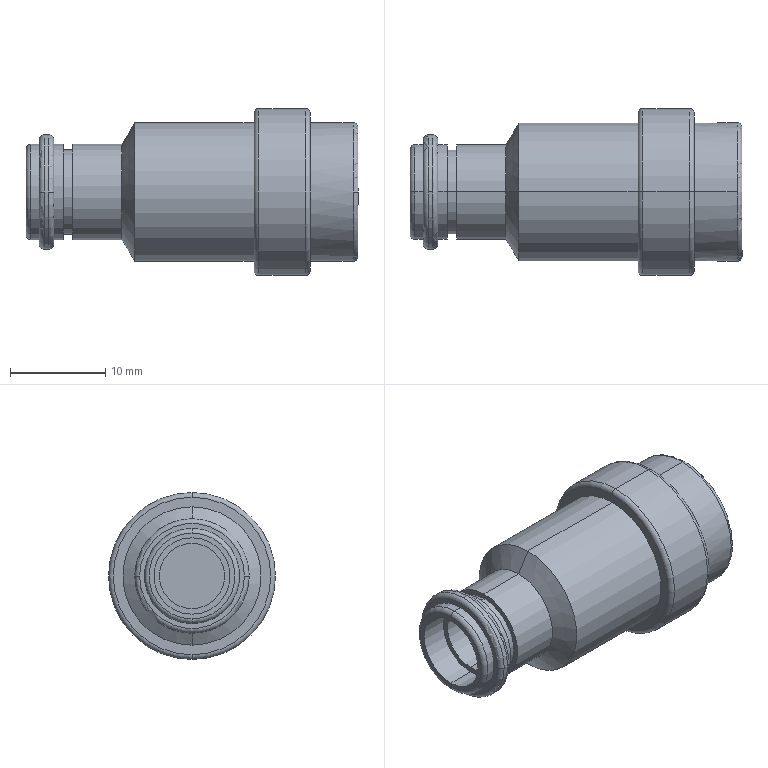Part | STEP file | 航插-2 | 1 solid | 57 faces | box 34.8 x 17.5 x 17.5 mm | volume 1736 mm3 | cylinder 28 | plane 13 | torus 12 | cone 4 | commonest cylinder face diameters 10 x6 8 x4 12.5 x4 14.5 x4 6.852 x2 8.852 x2
STEP:
#1=CARTESIAN_POINT('',(11.412,0.,-7.25));
#2=VERTEX_POINT('',#1);
#3=CARTESIAN_POINT('',(11.412,0.,7.25));
#4=VERTEX_POINT('',#3);
#5=CARTESIAN_POINT('',(11.412,0.,0.));
#6=DIRECTION('',(1.,0.,0.));
#7=DIRECTION('',(0.,0.,-1.));
#8=AXIS2_PLACEMENT_3D('',#5,#6,#7);
#9=CIRCLE('',#8,7.25);
#10=EDGE_CURVE('',#2,#4,#9,.T.);
#11=ORIENTED_EDGE('',*,*,#10,.T.);
#12=CARTESIAN_POINT('',(23.9,0.,7.25));
#13=VERTEX_POINT('',#12);
#14=CARTESIAN_POINT('',(34.8,0.,7.25));
#15=DIRECTION('',(1.,0.,0.));
#16=VECTOR('',#15,1000.);
#17=LINE('',#14,#16);
#18=EDGE_CURVE('',#4,#13,#17,.T.);
#19=ORIENTED_EDGE('',*,*,#18,.T.);
#20=CARTESIAN_POINT('',(23.9,0.,-7.25));
#21=VERTEX_POINT('',#20);
#22=CARTESIAN_POINT('',(23.9,0.,0.));
#23=DIRECTION('',(-1.,0.,0.));
#24=DIRECTION('',(0.,0.,-1.));
#25=AXIS2_PLACEMENT_3D('',#22,#23,#24);
#26=CIRCLE('',#25,7.25);
#27=EDGE_CURVE('',#13,#21,#26,.T.);
#28=ORIENTED_EDGE('',*,*,#27,.T.);
#29=CARTESIAN_POINT('',(34.8,0.,-7.25));
#30=DIRECTION('',(1.,0.,0.));
#31=VECTOR('',#30,1000.);
#32=LINE('',#29,#31);
#33=EDGE_CURVE('',#2,#21,#32,.T.);
#34=ORIENTED_EDGE('',*,*,#33,.F.);
#35=EDGE_LOOP('',(#11,#19,#28,#34));
#36=FACE_OUTER_BOUND('',#35,.T.);
#37=CARTESIAN_POINT('',(34.8,0.,0.));
#38=DIRECTION('',(1.,0.,0.));
#39=DIRECTION('',(0.,0.,-1.));
#40=AXIS2_PLACEMENT_3D('',#37,#38,#39);
#41=CYLINDRICAL_SURFACE('',#40,7.25);
#42=ADVANCED_FACE('',(#36),#41,.T.);
#43=CARTESIAN_POINT('',(10.05,0.,-5.));
#44=VERTEX_POINT('',#43);
#45=CARTESIAN_POINT('',(10.05,0.,5.));
#46=VERTEX_POINT('',#45);
#47=CARTESIAN_POINT('',(10.05,0.,0.));
#48=DIRECTION('',(1.,0.,0.));
#49=DIRECTION('',(0.,0.,-1.));
#50=AXIS2_PLACEMENT_3D('',#47,#48,#49);
#51=CIRCLE('',#50,5.);
#52=EDGE_CURVE('',#44,#46,#51,.T.);
#53=ORIENTED_EDGE('',*,*,#52,.T.);
#54=CARTESIAN_POINT('',(11.412,0.,7.25));
#55=DIRECTION('',(0.5179,0.,0.8555));
#56=VECTOR('',#55,1000.);
#57=LINE('',#54,#56);
#58=EDGE_CURVE('',#46,#4,#57,.T.);
#59=ORIENTED_EDGE('',*,*,#58,.T.);
#60=ORIENTED_EDGE('',*,*,#10,.F.);
#61=CARTESIAN_POINT('',(11.412,0.,-7.25));
#62=DIRECTION('',(0.5179,0.,-0.8555));
#63=VECTOR('',#62,1000.);
#64=LINE('',#61,#63);
#65=EDGE_CURVE('',#44,#2,#64,.T.);
#66=ORIENTED_EDGE('',*,*,#65,.F.);
#67=EDGE_LOOP('',(#53,#59,#60,#66));
#68=FACE_OUTER_BOUND('',#67,.T.);
#69=CARTESIAN_POINT('',(11.412,0.,0.));
#70=DIRECTION('',(1.,0.,0.));
#71=DIRECTION('',(0.,0.,-1.));
#72=AXIS2_PLACEMENT_3D('',#69,#70,#71);
#73=CONICAL_SURFACE('',#72,7.25,1.026);
#74=ADVANCED_FACE('',(#68),#73,.T.);
#75=CARTESIAN_POINT('',(24.4,0.,8.75));
#76=VERTEX_POINT('',#75);
#77=CARTESIAN_POINT('',(24.4,0.,-8.75));
#78=VERTEX_POINT('',#77);
#79=CARTESIAN_POINT('',(24.4,0.,0.));
#80=DIRECTION('',(-1.,0.,0.));
#81=DIRECTION('',(0.,0.,-1.));
#82=AXIS2_PLACEMENT_3D('',#79,#80,#81);
#83=CIRCLE('',#82,8.75);
#84=EDGE_CURVE('',#76,#78,#83,.T.);
#85=ORIENTED_EDGE('',*,*,#84,.T.);
#86=CARTESIAN_POINT('',(23.9,0.,-8.25));
#87=VERTEX_POINT('',#86);
#88=CARTESIAN_POINT('',(24.4,0.,-8.25));
#89=DIRECTION('',(0.,1.,0.));
#90=DIRECTION('',(0.,0.,1.));
#91=AXIS2_PLACEMENT_3D('',#88,#89,#90);
#92=CIRCLE('',#91,0.5);
#93=EDGE_CURVE('',#78,#87,#92,.T.);
#94=ORIENTED_EDGE('',*,*,#93,.T.);
#95=CARTESIAN_POINT('',(23.9,0.,8.25));
#96=VERTEX_POINT('',#95);
#97=CARTESIAN_POINT('',(23.9,0.,0.));
#98=DIRECTION('',(-1.,0.,0.));
#99=DIRECTION('',(0.,0.,1.));
#100=AXIS2_PLACEMENT_3D('',#97,#98,#99);
#101=CIRCLE('',#100,8.25);
#102=EDGE_CURVE('',#96,#87,#101,.T.);
#103=ORIENTED_EDGE('',*,*,#102,.F.);
#104=CARTESIAN_POINT('',(24.4,0.,8.25));
#105=DIRECTION('',(0.,-1.,0.));
#106=DIRECTION('',(0.,0.,-1.));
#107=AXIS2_PLACEMENT_3D('',#104,#105,#106);
#108=CIRCLE('',#107,0.5);
#109=EDGE_CURVE('',#76,#96,#108,.T.);
#110=ORIENTED_EDGE('',*,*,#109,.F.);
#111=EDGE_LOOP('',(#85,#94,#103,#110));
#112=FACE_OUTER_BOUND('',#111,.T.);
#113=CARTESIAN_POINT('',(24.4,0.,0.));
#114=DIRECTION('',(-1.,0.,0.));
#115=DIRECTION('',(0.,0.,1.));
#116=AXIS2_PLACEMENT_3D('',#113,#114,#115);
#117=TOROIDAL_SURFACE('',#116,8.25,0.5);
#118=ADVANCED_FACE('',(#112),#117,.T.);
#119=CARTESIAN_POINT('',(4.9,0.,-5.));
#120=VERTEX_POINT('',#119);
#121=CARTESIAN_POINT('',(4.9,0.,5.));
#122=VERTEX_POINT('',#121);
#123=CARTESIAN_POINT('',(4.9,0.,0.));
#124=DIRECTION('',(1.,0.,0.));
#125=DIRECTION('',(0.,0.,-1.));
#126=AXIS2_PLACEMENT_3D('',#123,#124,#125);
#127=CIRCLE('',#126,5.);
#128=EDGE_CURVE('',#120,#122,#127,.T.);
#129=ORIENTED_EDGE('',*,*,#128,.T.);
#130=CARTESIAN_POINT('',(34.8,0.,5.));
#131=DIRECTION('',(1.,0.,0.));
#132=VECTOR('',#131,1000.);
#133=LINE('',#130,#132);
#134=EDGE_CURVE('',#122,#46,#133,.T.);
#135=ORIENTED_EDGE('',*,*,#134,.T.);
#136=ORIENTED_EDGE('',*,*,#52,.F.);
#137=CARTESIAN_POINT('',(34.8,0.,-5.));
#138=DIRECTION('',(1.,0.,0.));
#139=VECTOR('',#138,1000.);
#140=LINE('',#137,#139);
#141=EDGE_CURVE('',#120,#44,#140,.T.);
#142=ORIENTED_EDGE('',*,*,#141,.F.);
#143=EDGE_LOOP('',(#129,#135,#136,#142));
#144=FACE_OUTER_BOUND('',#143,.T.);
#145=CARTESIAN_POINT('',(34.8,0.,0.));
#146=DIRECTION('',(1.,0.,0.));
#147=DIRECTION('',(0.,0.,-1.));
#148=AXIS2_PLACEMENT_3D('',#145,#146,#147);
#149=CYLINDRICAL_SURFACE('',#148,5.);
#150=ADVANCED_FACE('',(#144),#149,.T.);
#151=ORIENTED_EDGE('',*,*,#84,.F.);
#152=CARTESIAN_POINT('',(29.3,0.,8.75));
#153=VERTEX_POINT('',#152);
#154=CARTESIAN_POINT('',(34.8,0.,8.75));
#155=DIRECTION('',(1.,0.,0.));
#156=VECTOR('',#155,1000.);
#157=LINE('',#154,#156);
#158=EDGE_CURVE('',#76,#153,#157,.T.);
#159=ORIENTED_EDGE('',*,*,#158,.T.);
#160=CARTESIAN_POINT('',(29.3,0.,-8.75));
#161=VERTEX_POINT('',#160);
#162=CARTESIAN_POINT('',(29.3,0.,0.));
#163=DIRECTION('',(-1.,0.,0.));
#164=DIRECTION('',(0.,0.,-1.));
#165=AXIS2_PLACEMENT_3D('',#162,#163,#164);
#166=CIRCLE('',#165,8.75);
#167=EDGE_CURVE('',#153,#161,#166,.T.);
#168=ORIENTED_EDGE('',*,*,#167,.T.);
#169=CARTESIAN_POINT('',(34.8,0.,-8.75));
#170=DIRECTION('',(1.,0.,0.));
#171=VECTOR('',#170,1000.);
#172=LINE('',#169,#171);
#173=EDGE_CURVE('',#78,#161,#172,.T.);
#174=ORIENTED_EDGE('',*,*,#173,.F.);
#175=EDGE_LOOP('',(#151,#159,#168,#174));
#176=FACE_OUTER_BOUND('',#175,.T.);
#177=CARTESIAN_POINT('',(34.8,0.,0.));
#178=DIRECTION('',(1.,0.,0.));
#179=DIRECTION('',(0.,0.,-1.));
#180=AXIS2_PLACEMENT_3D('',#177,#178,#179);
#181=CYLINDRICAL_SURFACE('',#180,8.75);
#182=ADVANCED_FACE('',(#176),#181,.T.);
#183=ORIENTED_EDGE('',*,*,#167,.F.);
#184=CARTESIAN_POINT('',(29.8,0.,8.25));
#185=VERTEX_POINT('',#184);
#186=CARTESIAN_POINT('',(29.3,0.,8.25));
#187=DIRECTION('',(0.,1.,0.));
#188=DIRECTION('',(0.,0.,1.));
#189=AXIS2_PLACEMENT_3D('',#186,#187,#188);
#190=CIRCLE('',#189,0.5);
#191=EDGE_CURVE('',#153,#185,#190,.T.);
#192=ORIENTED_EDGE('',*,*,#191,.T.);
#193=CARTESIAN_POINT('',(29.8,0.,-8.25));
#194=VERTEX_POINT('',#193);
#195=CARTESIAN_POINT('',(29.8,0.,0.));
#196=DIRECTION('',(-1.,0.,0.));
#197=DIRECTION('',(0.,0.,-1.));
#198=AXIS2_PLACEMENT_3D('',#195,#196,#197);
#199=CIRCLE('',#198,8.25);
#200=EDGE_CURVE('',#185,#194,#199,.T.);
#201=ORIENTED_EDGE('',*,*,#200,.T.);
#202=CARTESIAN_POINT('',(29.3,0.,-8.25));
#203=DIRECTION('',(0.,-1.,0.));
#204=DIRECTION('',(0.,0.,-1.));
#205=AXIS2_PLACEMENT_3D('',#202,#203,#204);
#206=CIRCLE('',#205,0.5);
#207=EDGE_CURVE('',#161,#194,#206,.T.);
#208=ORIENTED_EDGE('',*,*,#207,.F.);
#209=EDGE_LOOP('',(#183,#192,#201,#208));
#210=FACE_OUTER_BOUND('',#209,.T.);
#211=CARTESIAN_POINT('',(29.3,0.,0.));
#212=DIRECTION('',(1.,0.,0.));
#213=DIRECTION('',(0.,0.,-1.));
#214=AXIS2_PLACEMENT_3D('',#211,#212,#213);
#215=TOROIDAL_SURFACE('',#214,8.25,0.5);
#216=ADVANCED_FACE('',(#210),#215,.T.);
#217=CARTESIAN_POINT('',(3.9,0.,-4.426));
#218=VERTEX_POINT('',#217);
#219=CARTESIAN_POINT('',(3.9,0.,4.426));
#220=VERTEX_POINT('',#219);
#221=CARTESIAN_POINT('',(3.9,0.,0.));
#222=DIRECTION('',(1.,0.,0.));
#223=DIRECTION('',(0.,0.,-1.));
#224=AXIS2_PLACEMENT_3D('',#221,#222,#223);
#225=CIRCLE('',#224,4.426);
#226=EDGE_CURVE('',#218,#220,#225,.T.);
#227=ORIENTED_EDGE('',*,*,#226,.T.);
#228=CARTESIAN_POINT('',(4.9,0.,4.426));
#229=VERTEX_POINT('',#228);
#230=CARTESIAN_POINT('',(34.8,0.,4.426));
#231=DIRECTION('',(1.,0.,0.));
#232=VECTOR('',#231,1000.);
#233=LINE('',#230,#232);
#234=EDGE_CURVE('',#220,#229,#233,.T.);
#235=ORIENTED_EDGE('',*,*,#234,.T.);
#236=CARTESIAN_POINT('',(4.9,0.,-4.426));
#237=VERTEX_POINT('',#236);
#238=CARTESIAN_POINT('',(4.9,0.,0.));
#239=DIRECTION('',(1.,0.,0.));
#240=DIRECTION('',(0.,0.,-1.));
#241=AXIS2_PLACEMENT_3D('',#238,#239,#240);
#242=CIRCLE('',#241,4.426);
#243=EDGE_CURVE('',#237,#229,#242,.T.);
#244=ORIENTED_EDGE('',*,*,#243,.F.);
#245=CARTESIAN_POINT('',(34.8,0.,-4.426));
#246=DIRECTION('',(1.,0.,0.));
#247=VECTOR('',#246,1000.);
#248=LINE('',#245,#247);
#249=EDGE_CURVE('',#218,#237,#248,.T.);
#250=ORIENTED_EDGE('',*,*,#249,.F.);
#251=EDGE_LOOP('',(#227,#235,#244,#250));
#252=FACE_OUTER_BOUND('',#251,.T.);
#253=CARTESIAN_POINT('',(34.8,0.,0.));
#254=DIRECTION('',(1.,0.,0.));
#255=DIRECTION('',(0.,0.,-1.));
#256=AXIS2_PLACEMENT_3D('',#253,#254,#255);
#257=CYLINDRICAL_SURFACE('',#256,4.426);
#258=ADVANCED_FACE('',(#252),#257,.T.);
#259=CARTESIAN_POINT('',(29.8,0.,7.25));
#260=VERTEX_POINT('',#259);
#261=CARTESIAN_POINT('',(29.8,0.,-7.25));
#262=VERTEX_POINT('',#261);
#263=CARTESIAN_POINT('',(29.8,0.,0.));
#264=DIRECTION('',(-1.,0.,0.));
#265=DIRECTION('',(0.,0.,-1.));
#266=AXIS2_PLACEMENT_3D('',#263,#264,#265);
#267=CIRCLE('',#266,7.25);
#268=EDGE_CURVE('',#260,#262,#267,.T.);
#269=ORIENTED_EDGE('',*,*,#268,.F.);
#270=CARTESIAN_POINT('',(34.3,0.,7.25));
#271=VERTEX_POINT('',#270);
#272=CARTESIAN_POINT('',(34.8,0.,7.25));
#273=DIRECTION('',(1.,0.,0.));
#274=VECTOR('',#273,1000.);
#275=LINE('',#272,#274);
#276=EDGE_CURVE('',#260,#271,#275,.T.);
#277=ORIENTED_EDGE('',*,*,#276,.T.);
#278=CARTESIAN_POINT('',(34.3,7.25,0.));
#279=VERTEX_POINT('',#278);
#280=CARTESIAN_POINT('',(34.3,0.,0.));
#281=DIRECTION('',(-1.,0.,0.));
#282=DIRECTION('',(0.,0.,-1.));
#283=AXIS2_PLACEMENT_3D('',#280,#281,#282);
#284=CIRCLE('',#283,7.25);
#285=EDGE_CURVE('',#271,#279,#284,.T.);
#286=ORIENTED_EDGE('',*,*,#285,.T.);
#287=CARTESIAN_POINT('',(34.3,0.,-7.25));
#288=VERTEX_POINT('',#287);
#289=CARTESIAN_POINT('',(34.3,0.,0.));
#290=DIRECTION('',(-1.,0.,0.));
#291=DIRECTION('',(0.,0.,-1.));
#292=AXIS2_PLACEMENT_3D('',#289,#290,#291);
#293=CIRCLE('',#292,7.25);
#294=EDGE_CURVE('',#279,#288,#293,.T.);
#295=ORIENTED_EDGE('',*,*,#294,.T.);
#296=CARTESIAN_POINT('',(34.8,0.,-7.25));
#297=DIRECTION('',(1.,0.,0.));
#298=VECTOR('',#297,1000.);
#299=LINE('',#296,#298);
#300=EDGE_CURVE('',#262,#288,#299,.T.);
#301=ORIENTED_EDGE('',*,*,#300,.F.);
#302=EDGE_LOOP('',(#269,#277,#286,#295,#301));
#303=FACE_OUTER_BOUND('',#302,.T.);
#304=CARTESIAN_POINT('',(34.8,0.,0.));
#305=DIRECTION('',(1.,0.,0.));
#306=DIRECTION('',(0.,0.,-1.));
#307=AXIS2_PLACEMENT_3D('',#304,#305,#306);
#308=CYLINDRICAL_SURFACE('',#307,7.25);
#309=ADVANCED_FACE('',(#303),#308,.T.);
#310=CARTESIAN_POINT('',(2.9,0.,-5.));
#311=VERTEX_POINT('',#310);
#312=CARTESIAN_POINT('',(2.9,0.,5.));
#313=VERTEX_POINT('',#312);
#314=CARTESIAN_POINT('',(2.9,0.,0.));
#315=DIRECTION('',(1.,0.,0.));
#316=DIRECTION('',(0.,0.,-1.));
#317=AXIS2_PLACEMENT_3D('',#314,#315,#316);
#318=CIRCLE('',#317,5.);
#319=EDGE_CURVE('',#311,#313,#318,.T.);
#320=ORIENTED_EDGE('',*,*,#319,.T.);
#321=CARTESIAN_POINT('',(3.9,0.,5.));
#322=VERTEX_POINT('',#321);
#323=CARTESIAN_POINT('',(34.8,0.,5.));
#324=DIRECTION('',(1.,0.,0.));
#325=VECTOR('',#324,1000.);
#326=LINE('',#323,#325);
#327=EDGE_CURVE('',#313,#322,#326,.T.);
#328=ORIENTED_EDGE('',*,*,#327,.T.);
#329=CARTESIAN_POINT('',(3.9,0.,-5.));
#330=VERTEX_POINT('',#329);
#331=CARTESIAN_POINT('',(3.9,0.,0.));
#332=DIRECTION('',(1.,0.,0.));
#333=DIRECTION('',(0.,0.,-1.));
#334=AXIS2_PLACEMENT_3D('',#331,#332,#333);
#335=CIRCLE('',#334,5.);
#336=EDGE_CURVE('',#330,#322,#335,.T.);
#337=ORIENTED_EDGE('',*,*,#336,.F.);
#338=CARTESIAN_POINT('',(34.8,0.,-5.));
#339=DIRECTION('',(1.,0.,0.));
#340=VECTOR('',#339,1000.);
#341=LINE('',#338,#340);
#342=EDGE_CURVE('',#311,#330,#341,.T.);
#343=ORIENTED_EDGE('',*,*,#342,.F.);
#344=EDGE_LOOP('',(#320,#328,#337,#343));
#345=FACE_OUTER_BOUND('',#344,.T.);
#346=CARTESIAN_POINT('',(34.8,0.,0.));
#347=DIRECTION('',(1.,0.,0.));
#348=DIRECTION('',(0.,0.,-1.));
#349=AXIS2_PLACEMENT_3D('',#346,#347,#348);
#350=CYLINDRICAL_SURFACE('',#349,5.);
#351=ADVANCED_FACE('',(#345),#350,.T.);
#352=CARTESIAN_POINT('',(34.3,-7.25,0.));
#353=VERTEX_POINT('',#352);
#354=CARTESIAN_POINT('',(34.3,0.,0.));
#355=DIRECTION('',(-1.,0.,0.));
#356=DIRECTION('',(0.,0.,-1.));
#357=AXIS2_PLACEMENT_3D('',#354,#355,#356);
#358=CIRCLE('',#357,7.25);
#359=EDGE_CURVE('',#353,#271,#358,.T.);
#360=ORIENTED_EDGE('',*,*,#359,.F.);
#361=CARTESIAN_POINT('',(34.8,-6.75,0.));
#362=VERTEX_POINT('',#361);
#363=CARTESIAN_POINT('',(34.3,-6.75,0.));
#364=DIRECTION('',(0.,0.,1.));
#365=DIRECTION('',(0.,-1.,0.));
#366=AXIS2_PLACEMENT_3D('',#363,#364,#365);
#367=CIRCLE('',#366,0.5);
#368=EDGE_CURVE('',#353,#362,#367,.T.);
#369=ORIENTED_EDGE('',*,*,#368,.T.);
#370=CARTESIAN_POINT('',(34.8,6.75,0.));
#371=VERTEX_POINT('',#370);
#372=CARTESIAN_POINT('',(34.8,0.,0.));
#373=DIRECTION('',(-1.,0.,0.));
#374=DIRECTION('',(0.,1.,0.));
#375=AXIS2_PLACEMENT_3D('',#372,#373,#374);
#376=CIRCLE('',#375,6.75);
#377=EDGE_CURVE('',#362,#371,#376,.T.);
#378=ORIENTED_EDGE('',*,*,#377,.T.);
#379=CARTESIAN_POINT('',(34.3,6.75,0.));
#380=DIRECTION('',(0.,0.,-1.));
#381=DIRECTION('',(-1.,0.,0.));
#382=AXIS2_PLACEMENT_3D('',#379,#380,#381);
#383=CIRCLE('',#382,0.5);
#384=EDGE_CURVE('',#279,#371,#383,.T.);
#385=ORIENTED_EDGE('',*,*,#384,.F.);
#386=ORIENTED_EDGE('',*,*,#285,.F.);
#387=EDGE_LOOP('',(#360,#369,#378,#385,#386));
#388=FACE_OUTER_BOUND('',#387,.T.);
#389=CARTESIAN_POINT('',(34.3,0.,0.));
#390=DIRECTION('',(1.,0.,0.));
#391=DIRECTION('',(0.,1.,0.));
#392=AXIS2_PLACEMENT_3D('',#389,#390,#391);
#393=TOROIDAL_SURFACE('',#392,6.75,0.5);
#394=ADVANCED_FACE('',(#388),#393,.T.);
#395=CARTESIAN_POINT('',(2.4,0.,6.));
#396=VERTEX_POINT('',#395);
#397=CARTESIAN_POINT('',(2.4,-6.,0.));
#398=VERTEX_POINT('',#397);
#399=CARTESIAN_POINT('',(2.4,0.,0.));
#400=DIRECTION('',(1.,0.,0.));
#401=DIRECTION('',(0.,0.,1.));
#402=AXIS2_PLACEMENT_3D('',#399,#400,#401);
#403=CIRCLE('',#402,6.);
#404=EDGE_CURVE('',#396,#398,#403,.T.);
#405=ORIENTED_EDGE('',*,*,#404,.T.);
#406=CARTESIAN_POINT('',(2.9,-5.5,0.));
#407=VERTEX_POINT('',#406);
#408=CARTESIAN_POINT('',(2.4,-5.5,0.));
#409=DIRECTION('',(0.,0.,1.));
#410=DIRECTION('',(0.,-1.,0.));
#411=AXIS2_PLACEMENT_3D('',#408,#409,#410);
#412=CIRCLE('',#411,0.5);
#413=EDGE_CURVE('',#398,#407,#412,.T.);
#414=ORIENTED_EDGE('',*,*,#413,.T.);
#415=CARTESIAN_POINT('',(2.9,5.5,0.));
#416=VERTEX_POINT('',#415);
#417=CARTESIAN_POINT('',(2.9,0.,0.));
#418=DIRECTION('',(1.,0.,0.));
#419=DIRECTION('',(0.,1.,0.));
#420=AXIS2_PLACEMENT_3D('',#417,#418,#419);
#421=CIRCLE('',#420,5.5);
#422=EDGE_CURVE('',#416,#407,#421,.T.);
#423=ORIENTED_EDGE('',*,*,#422,.F.);
#424=CARTESIAN_POINT('',(2.4,6.,0.));
#425=VERTEX_POINT('',#424);
#426=CARTESIAN_POINT('',(2.4,5.5,0.));
#427=DIRECTION('',(0.,0.,-1.));
#428=DIRECTION('',(-1.,0.,0.));
#429=AXIS2_PLACEMENT_3D('',#426,#427,#428);
#430=CIRCLE('',#429,0.5);
#431=EDGE_CURVE('',#425,#416,#430,.T.);
#432=ORIENTED_EDGE('',*,*,#431,.F.);
#433=CARTESIAN_POINT('',(2.4,0.,0.));
#434=DIRECTION('',(1.,0.,0.));
#435=DIRECTION('',(0.,0.,1.));
#436=AXIS2_PLACEMENT_3D('',#433,#434,#435);
#437=CIRCLE('',#436,6.);
#438=EDGE_CURVE('',#425,#396,#437,.T.);
#439=ORIENTED_EDGE('',*,*,#438,.T.);
#440=EDGE_LOOP('',(#405,#414,#423,#432,#439));
#441=FACE_OUTER_BOUND('',#440,.T.);
#442=CARTESIAN_POINT('',(2.4,0.,0.));
#443=DIRECTION('',(1.,0.,0.));
#444=DIRECTION('',(0.,1.,0.));
#445=AXIS2_PLACEMENT_3D('',#442,#443,#444);
#446=TOROIDAL_SURFACE('',#445,5.5,0.5);
#447=ADVANCED_FACE('',(#441),#446,.T.);
#448=CARTESIAN_POINT('',(1.9,6.,0.));
#449=VERTEX_POINT('',#448);
#450=CARTESIAN_POINT('',(1.9,0.,6.));
#451=VERTEX_POINT('',#450);
#452=CARTESIAN_POINT('',(1.9,0.,0.));
#453=DIRECTION('',(1.,0.,0.));
#454=DIRECTION('',(0.,0.,-1.));
#455=AXIS2_PLACEMENT_3D('',#452,#453,#454);
#456=CIRCLE('',#455,6.);
#457=EDGE_CURVE('',#449,#451,#456,.T.);
#458=ORIENTED_EDGE('',*,*,#457,.T.);
#459=CARTESIAN_POINT('',(34.8,0.,6.));
#460=DIRECTION('',(1.,0.,0.));
#461=VECTOR('',#460,1000.);
#462=LINE('',#459,#461);
#463=EDGE_CURVE('',#451,#396,#462,.T.);
#464=ORIENTED_EDGE('',*,*,#463,.T.);
#465=ORIENTED_EDGE('',*,*,#438,.F.);
#466=CARTESIAN_POINT('',(2.4,0.,-6.));
#467=VERTEX_POINT('',#466);
#468=CARTESIAN_POINT('',(2.4,0.,0.));
#469=DIRECTION('',(1.,0.,0.));
#470=DIRECTION('',(0.,0.,1.));
#471=AXIS2_PLACEMENT_3D('',#468,#469,#470);
#472=CIRCLE('',#471,6.);
#473=EDGE_CURVE('',#467,#425,#472,.T.);
#474=ORIENTED_EDGE('',*,*,#473,.F.);
#475=CARTESIAN_POINT('',(1.9,0.,-6.));
#476=VERTEX_POINT('',#475);
#477=CARTESIAN_POINT('',(34.8,0.,-6.));
#478=DIRECTION('',(1.,0.,0.));
#479=VECTOR('',#478,1000.);
#480=LINE('',#477,#479);
#481=EDGE_CURVE('',#476,#467,#480,.T.);
#482=ORIENTED_EDGE('',*,*,#481,.F.);
#483=CARTESIAN_POINT('',(1.9,0.,0.));
#484=DIRECTION('',(1.,0.,0.));
#485=DIRECTION('',(0.,0.,-1.));
#486=AXIS2_PLACEMENT_3D('',#483,#484,#485);
#487=CIRCLE('',#486,6.);
#488=EDGE_CURVE('',#476,#449,#487,.T.);
#489=ORIENTED_EDGE('',*,*,#488,.T.);
#490=EDGE_LOOP('',(#458,#464,#465,#474,#482,#489));
#491=FACE_OUTER_BOUND('',#490,.T.);
#492=CARTESIAN_POINT('',(34.8,0.,0.));
#493=DIRECTION('',(1.,0.,0.));
#494=DIRECTION('',(0.,0.,-1.));
#495=AXIS2_PLACEMENT_3D('',#492,#493,#494);
#496=CYLINDRICAL_SURFACE('',#495,6.);
#497=ADVANCED_FACE('',(#491),#496,.T.);
#498=ORIENTED_EDGE('',*,*,#457,.F.);
#499=CARTESIAN_POINT('',(1.4,5.5,0.));
#500=VERTEX_POINT('',#499);
#501=CARTESIAN_POINT('',(1.9,5.5,0.));
#502=DIRECTION('',(0.,0.,1.));
#503=DIRECTION('',(0.,-1.,0.));
#504=AXIS2_PLACEMENT_3D('',#501,#502,#503);
#505=CIRCLE('',#504,0.5);
#506=EDGE_CURVE('',#449,#500,#505,.T.);
#507=ORIENTED_EDGE('',*,*,#506,.T.);
#508=CARTESIAN_POINT('',(1.4,-5.5,0.));
#509=VERTEX_POINT('',#508);
#510=CARTESIAN_POINT('',(1.4,0.,0.));
#511=DIRECTION('',(1.,0.,0.));
#512=DIRECTION('',(0.,-1.,0.));
#513=AXIS2_PLACEMENT_3D('',#510,#511,#512);
#514=CIRCLE('',#513,5.5);
#515=EDGE_CURVE('',#500,#509,#514,.T.);
#516=ORIENTED_EDGE('',*,*,#515,.T.);
#517=CARTESIAN_POINT('',(1.9,-6.,0.));
#518=VERTEX_POINT('',#517);
#519=CARTESIAN_POINT('',(1.9,-5.5,0.));
#520=DIRECTION('',(0.,0.,-1.));
#521=DIRECTION('',(-1.,0.,0.));
#522=AXIS2_PLACEMENT_3D('',#519,#520,#521);
#523=CIRCLE('',#522,0.5);
#524=EDGE_CURVE('',#518,#509,#523,.T.);
#525=ORIENTED_EDGE('',*,*,#524,.F.);
#526=CARTESIAN_POINT('',(1.9,0.,0.));
#527=DIRECTION('',(1.,0.,0.));
#528=DIRECTION('',(0.,0.,-1.));
#529=AXIS2_PLACEMENT_3D('',#526,#527,#528);
#530=CIRCLE('',#529,6.);
#531=EDGE_CURVE('',#451,#518,#530,.T.);
#532=ORIENTED_EDGE('',*,*,#531,.F.);
#533=EDGE_LOOP('',(#498,#507,#516,#525,#532));
#534=FACE_OUTER_BOUND('',#533,.T.);
#535=CARTESIAN_POINT('',(1.9,0.,0.));
#536=DIRECTION('',(-1.,0.,0.));
#537=DIRECTION('',(0.,-1.,0.));
#538=AXIS2_PLACEMENT_3D('',#535,#536,#537);
#539=TOROIDAL_SURFACE('',#538,5.5,0.5);
#540=ADVANCED_FACE('',(#534),#539,.T.);
#541=CARTESIAN_POINT('',(0.5,0.,-5.));
#542=VERTEX_POINT('',#541);
#543=CARTESIAN_POINT('',(0.5,0.,5.));
#544=VERTEX_POINT('',#543);
#545=CARTESIAN_POINT('',(0.5,0.,0.));
#546=DIRECTION('',(1.,0.,0.));
#547=DIRECTION('',(0.,0.,-1.));
#548=AXIS2_PLACEMENT_3D('',#545,#546,#547);
#549=CIRCLE('',#548,5.);
#550=EDGE_CURVE('',#542,#544,#549,.T.);
#551=ORIENTED_EDGE('',*,*,#550,.T.);
#552=CARTESIAN_POINT('',(1.4,0.,5.));
#553=VERTEX_POINT('',#552);
#554=CARTESIAN_POINT('',(34.8,0.,5.));
#555=DIRECTION('',(1.,0.,0.));
#556=VECTOR('',#555,1000.);
#557=LINE('',#554,#556);
#558=EDGE_CURVE('',#544,#553,#557,.T.);
#559=ORIENTED_EDGE('',*,*,#558,.T.);
#560=CARTESIAN_POINT('',(1.4,0.,-5.));
#561=VERTEX_POINT('',#560);
#562=CARTESIAN_POINT('',(1.4,0.,0.));
#563=DIRECTION('',(1.,0.,0.));
#564=DIRECTION('',(0.,0.,-1.));
#565=AXIS2_PLACEMENT_3D('',#562,#563,#564);
#566=CIRCLE('',#565,5.);
#567=EDGE_CURVE('',#561,#553,#566,.T.);
#568=ORIENTED_EDGE('',*,*,#567,.F.);
#569=CARTESIAN_POINT('',(34.8,0.,-5.));
#570=DIRECTION('',(1.,0.,0.));
#571=VECTOR('',#570,1000.);
#572=LINE('',#569,#571);
#573=EDGE_CURVE('',#542,#561,#572,.T.);
#574=ORIENTED_EDGE('',*,*,#573,.F.);
#575=EDGE_LOOP('',(#551,#559,#568,#574));
#576=FACE_OUTER_BOUND('',#575,.T.);
#577=CARTESIAN_POINT('',(34.8,0.,0.));
#578=DIRECTION('',(1.,0.,0.));
#579=DIRECTION('',(0.,0.,-1.));
#580=AXIS2_PLACEMENT_3D('',#577,#578,#579);
#581=CYLINDRICAL_SURFACE('',#580,5.);
#582=ADVANCED_FACE('',(#576),#581,.T.);
#583=ORIENTED_EDGE('',*,*,#550,.F.);
#584=CARTESIAN_POINT('',(0.,0.,-4.5));
#585=VERTEX_POINT('',#584);
#586=CARTESIAN_POINT('',(0.5,0.,-4.5));
#587=DIRECTION('',(0.,1.,0.));
#588=DIRECTION('',(0.,0.,1.));
#589=AXIS2_PLACEMENT_3D('',#586,#587,#588);
#590=CIRCLE('',#589,0.5);
#591=EDGE_CURVE('',#542,#585,#590,.T.);
#592=ORIENTED_EDGE('',*,*,#591,.T.);
#593=CARTESIAN_POINT('',(0.,0.,4.5));
#594=VERTEX_POINT('',#593);
#595=CARTESIAN_POINT('',(0.,0.,0.));
#596=DIRECTION('',(1.,0.,0.));
#597=DIRECTION('',(0.,0.,1.));
#598=AXIS2_PLACEMENT_3D('',#595,#596,#597);
#599=CIRCLE('',#598,4.5);
#600=EDGE_CURVE('',#585,#594,#599,.T.);
#601=ORIENTED_EDGE('',*,*,#600,.T.);
#602=CARTESIAN_POINT('',(0.5,0.,4.5));
#603=DIRECTION('',(0.,-1.,0.));
#604=DIRECTION('',(0.,0.,-1.));
#605=AXIS2_PLACEMENT_3D('',#602,#603,#604);
#606=CIRCLE('',#605,0.5);
#607=EDGE_CURVE('',#544,#594,#606,.T.);
#608=ORIENTED_EDGE('',*,*,#607,.F.);
#609=EDGE_LOOP('',(#583,#592,#601,#608));
#610=FACE_OUTER_BOUND('',#609,.T.);
#611=CARTESIAN_POINT('',(0.5,0.,0.));
#612=DIRECTION('',(-1.,0.,0.));
#613=DIRECTION('',(0.,0.,1.));
#614=AXIS2_PLACEMENT_3D('',#611,#612,#613);
#615=TOROIDAL_SURFACE('',#614,4.5,0.5);
#616=ADVANCED_FACE('',(#610),#615,.T.);
#617=CARTESIAN_POINT('',(0.,0.,4.));
#618=VERTEX_POINT('',#617);
#619=CARTESIAN_POINT('',(0.,0.,-4.));
#620=VERTEX_POINT('',#619);
#621=CARTESIAN_POINT('',(0.,0.,0.));
#622=DIRECTION('',(1.,0.,0.));
#623=DIRECTION('',(0.,0.,-1.));
#624=AXIS2_PLACEMENT_3D('',#621,#622,#623);
#625=CIRCLE('',#624,4.);
#626=EDGE_CURVE('',#618,#620,#625,.T.);
#627=ORIENTED_EDGE('',*,*,#626,.F.);
#628=CARTESIAN_POINT('',(2.9,0.,4.));
#629=VERTEX_POINT('',#628);
#630=CARTESIAN_POINT('',(34.8,0.,4.));
#631=DIRECTION('',(1.,0.,0.));
#632=VECTOR('',#631,1000.);
#633=LINE('',#630,#632);
#634=EDGE_CURVE('',#618,#629,#633,.T.);
#635=ORIENTED_EDGE('',*,*,#634,.T.);
#636=CARTESIAN_POINT('',(2.9,0.,-4.));
#637=VERTEX_POINT('',#636);
#638=CARTESIAN_POINT('',(2.9,0.,0.));
#639=DIRECTION('',(-1.,0.,0.));
#640=DIRECTION('',(0.,0.,-1.));
#641=AXIS2_PLACEMENT_3D('',#638,#639,#640);
#642=CIRCLE('',#641,4.);
#643=EDGE_CURVE('',#637,#629,#642,.T.);
#644=ORIENTED_EDGE('',*,*,#643,.F.);
#645=CARTESIAN_POINT('',(34.8,0.,-4.));
#646=DIRECTION('',(1.,0.,0.));
#647=VECTOR('',#646,1000.);
#648=LINE('',#645,#647);
#649=EDGE_CURVE('',#620,#637,#648,.T.);
#650=ORIENTED_EDGE('',*,*,#649,.F.);
#651=EDGE_LOOP('',(#627,#635,#644,#650));
#652=FACE_OUTER_BOUND('',#651,.T.);
#653=CARTESIAN_POINT('',(34.8,0.,0.));
#654=DIRECTION('',(1.,0.,0.));
#655=DIRECTION('',(0.,0.,-1.));
#656=AXIS2_PLACEMENT_3D('',#653,#654,#655);
#657=CYLINDRICAL_SURFACE('',#656,4.);
#658=ADVANCED_FACE('',(#652),#657,.F.);
#659=CARTESIAN_POINT('',(2.9,0.,-3.426));
#660=VERTEX_POINT('',#659);
#661=CARTESIAN_POINT('',(2.9,0.,3.426));
#662=VERTEX_POINT('',#661);
#663=CARTESIAN_POINT('',(2.9,0.,0.));
#664=DIRECTION('',(-1.,0.,0.));
#665=DIRECTION('',(0.,0.,-1.));
#666=AXIS2_PLACEMENT_3D('',#663,#664,#665);
#667=CIRCLE('',#666,3.426);
#668=EDGE_CURVE('',#660,#662,#667,.T.);
#669=ORIENTED_EDGE('',*,*,#668,.T.);
#670=CARTESIAN_POINT('',(5.9,0.,3.426));
#671=VERTEX_POINT('',#670);
#672=CARTESIAN_POINT('',(34.8,0.,3.426));
#673=DIRECTION('',(1.,0.,0.));
#674=VECTOR('',#673,1000.);
#675=LINE('',#672,#674);
#676=EDGE_CURVE('',#662,#671,#675,.T.);
#677=ORIENTED_EDGE('',*,*,#676,.T.);
#678=CARTESIAN_POINT('',(5.9,0.,-3.426));
#679=VERTEX_POINT('',#678);
#680=CARTESIAN_POINT('',(5.9,0.,0.));
#681=DIRECTION('',(-1.,0.,0.));
#682=DIRECTION('',(0.,0.,-1.));
#683=AXIS2_PLACEMENT_3D('',#680,#681,#682);
#684=CIRCLE('',#683,3.426);
#685=EDGE_CURVE('',#679,#671,#684,.T.);
#686=ORIENTED_EDGE('',*,*,#685,.F.);
#687=CARTESIAN_POINT('',(34.8,0.,-3.426));
#688=DIRECTION('',(1.,0.,0.));
#689=VECTOR('',#688,1000.);
#690=LINE('',#687,#689);
#691=EDGE_CURVE('',#660,#679,#690,.T.);
#692=ORIENTED_EDGE('',*,*,#691,.F.);
#693=EDGE_LOOP('',(#669,#677,#686,#692));
#694=FACE_OUTER_BOUND('',#693,.T.);
#695=CARTESIAN_POINT('',(34.8,0.,0.));
#696=DIRECTION('',(1.,0.,0.));
#697=DIRECTION('',(0.,0.,-1.));
#698=AXIS2_PLACEMENT_3D('',#695,#696,#697);
#699=CYLINDRICAL_SURFACE('',#698,3.426);
#700=ADVANCED_FACE('',(#694),#699,.F.);
#701=CARTESIAN_POINT('',(5.9,0.,-4.));
#702=VERTEX_POINT('',#701);
#703=CARTESIAN_POINT('',(5.9,0.,4.));
#704=VERTEX_POINT('',#703);
#705=CARTESIAN_POINT('',(5.9,0.,0.));
#706=DIRECTION('',(-1.,0.,0.));
#707=DIRECTION('',(0.,0.,-1.));
#708=AXIS2_PLACEMENT_3D('',#705,#706,#707);
#709=CIRCLE('',#708,4.);
#710=EDGE_CURVE('',#702,#704,#709,.T.);
#711=ORIENTED_EDGE('',*,*,#710,.T.);
#712=CARTESIAN_POINT('',(10.614,0.,4.));
#713=VERTEX_POINT('',#712);
#714=CARTESIAN_POINT('',(34.8,0.,4.));
#715=DIRECTION('',(1.,0.,0.));
#716=VECTOR('',#715,1000.);
#717=LINE('',#714,#716);
#718=EDGE_CURVE('',#704,#713,#717,.T.);
#719=ORIENTED_EDGE('',*,*,#718,.T.);
#720=CARTESIAN_POINT('',(10.614,-4.,0.));
#721=VERTEX_POINT('',#720);
#722=CARTESIAN_POINT('',(10.614,0.,0.));
#723=DIRECTION('',(-1.,0.,0.));
#724=DIRECTION('',(0.,0.,-1.));
#725=AXIS2_PLACEMENT_3D('',#722,#723,#724);
#726=CIRCLE('',#725,4.);
#727=EDGE_CURVE('',#721,#713,#726,.T.);
#728=ORIENTED_EDGE('',*,*,#727,.F.);
#729=CARTESIAN_POINT('',(10.614,0.,-4.));
#730=VERTEX_POINT('',#729);
#731=CARTESIAN_POINT('',(10.614,0.,0.));
#732=DIRECTION('',(-1.,0.,0.));
#733=DIRECTION('',(0.,0.,-1.));
#734=AXIS2_PLACEMENT_3D('',#731,#732,#733);
#735=CIRCLE('',#734,4.);
#736=EDGE_CURVE('',#730,#721,#735,.T.);
#737=ORIENTED_EDGE('',*,*,#736,.F.);
#738=CARTESIAN_POINT('',(34.8,0.,-4.));
#739=DIRECTION('',(1.,0.,0.));
#740=VECTOR('',#739,1000.);
#741=LINE('',#738,#740);
#742=EDGE_CURVE('',#702,#730,#741,.T.);
#743=ORIENTED_EDGE('',*,*,#742,.F.);
#744=EDGE_LOOP('',(#711,#719,#728,#737,#743));
#745=FACE_OUTER_BOUND('',#744,.T.);
#746=CARTESIAN_POINT('',(34.8,0.,0.));
#747=DIRECTION('',(1.,0.,0.));
#748=DIRECTION('',(0.,0.,-1.));
#749=AXIS2_PLACEMENT_3D('',#746,#747,#748);
#750=CYLINDRICAL_SURFACE('',#749,4.);
#751=ADVANCED_FACE('',(#745),#750,.F.);
#752=CARTESIAN_POINT('',(10.614,4.,0.));
#753=VERTEX_POINT('',#752);
#754=CARTESIAN_POINT('',(10.614,0.,0.));
#755=DIRECTION('',(-1.,0.,0.));
#756=DIRECTION('',(0.,0.,-1.));
#757=AXIS2_PLACEMENT_3D('',#754,#755,#756);
#758=CIRCLE('',#757,4.);
#759=EDGE_CURVE('',#753,#730,#758,.T.);
#760=ORIENTED_EDGE('',*,*,#759,.T.);
#761=ORIENTED_EDGE('',*,*,#736,.T.);
#762=CARTESIAN_POINT('',(11.976,-6.25,0.));
#763=VERTEX_POINT('',#762);
#764=CARTESIAN_POINT('',(11.976,-6.25,0.));
#765=DIRECTION('',(0.5179,-0.8555,0.));
#766=VECTOR('',#765,1000.);
#767=LINE('',#764,#766);
#768=EDGE_CURVE('',#721,#763,#767,.T.);
#769=ORIENTED_EDGE('',*,*,#768,.T.);
#770=CARTESIAN_POINT('',(11.976,0.,-6.25));
#771=VERTEX_POINT('',#770);
#772=CARTESIAN_POINT('',(11.976,0.,0.));
#773=DIRECTION('',(-1.,0.,0.));
#774=DIRECTION('',(0.,0.,-1.));
#775=AXIS2_PLACEMENT_3D('',#772,#773,#774);
#776=CIRCLE('',#775,6.25);
#777=EDGE_CURVE('',#771,#763,#776,.T.);
#778=ORIENTED_EDGE('',*,*,#777,.F.);
#779=CARTESIAN_POINT('',(11.976,6.25,0.));
#780=VERTEX_POINT('',#779);
#781=CARTESIAN_POINT('',(11.976,0.,0.));
#782=DIRECTION('',(-1.,0.,0.));
#783=DIRECTION('',(0.,0.,-1.));
#784=AXIS2_PLACEMENT_3D('',#781,#782,#783);
#785=CIRCLE('',#784,6.25);
#786=EDGE_CURVE('',#780,#771,#785,.T.);
#787=ORIENTED_EDGE('',*,*,#786,.F.);
#788=CARTESIAN_POINT('',(11.976,6.25,0.));
#789=DIRECTION('',(0.5179,0.8555,0.));
#790=VECTOR('',#789,1000.);
#791=LINE('',#788,#790);
#792=EDGE_CURVE('',#753,#780,#791,.T.);
#793=ORIENTED_EDGE('',*,*,#792,.F.);
#794=EDGE_LOOP('',(#760,#761,#769,#778,#787,#793));
#795=FACE_OUTER_BOUND('',#794,.T.);
#796=CARTESIAN_POINT('',(11.976,0.,0.));
#797=DIRECTION('',(1.,0.,0.));
#798=DIRECTION('',(0.,1.,0.));
#799=AXIS2_PLACEMENT_3D('',#796,#797,#798);
#800=CONICAL_SURFACE('',#799,6.25,1.026);
#801=ADVANCED_FACE('',(#795),#800,.F.);
#802=ORIENTED_EDGE('',*,*,#777,.T.);
#803=CARTESIAN_POINT('',(11.976,0.,6.25));
#804=VERTEX_POINT('',#803);
#805=CARTESIAN_POINT('',(11.976,0.,0.));
#806=DIRECTION('',(-1.,0.,0.));
#807=DIRECTION('',(0.,0.,-1.));
#808=AXIS2_PLACEMENT_3D('',#805,#806,#807);
#809=CIRCLE('',#808,6.25);
#810=EDGE_CURVE('',#763,#804,#809,.T.);
#811=ORIENTED_EDGE('',*,*,#810,.T.);
#812=CARTESIAN_POINT('',(24.9,0.,6.25));
#813=VERTEX_POINT('',#812);
#814=CARTESIAN_POINT('',(34.8,0.,6.25));
#815=DIRECTION('',(1.,0.,0.));
#816=VECTOR('',#815,1000.);
#817=LINE('',#814,#816);
#818=EDGE_CURVE('',#804,#813,#817,.T.);
#819=ORIENTED_EDGE('',*,*,#818,.T.);
#820=CARTESIAN_POINT('',(24.9,0.,-6.25));
#821=VERTEX_POINT('',#820);
#822=CARTESIAN_POINT('',(24.9,0.,0.));
#823=DIRECTION('',(-1.,0.,0.));
#824=DIRECTION('',(0.,0.,-1.));
#825=AXIS2_PLACEMENT_3D('',#822,#823,#824);
#826=CIRCLE('',#825,6.25);
#827=EDGE_CURVE('',#821,#813,#826,.T.);
#828=ORIENTED_EDGE('',*,*,#827,.F.);
#829=CARTESIAN_POINT('',(34.8,0.,-6.25));
#830=DIRECTION('',(1.,0.,0.));
#831=VECTOR('',#830,1000.);
#832=LINE('',#829,#831);
#833=EDGE_CURVE('',#771,#821,#832,.T.);
#834=ORIENTED_EDGE('',*,*,#833,.F.);
#835=EDGE_LOOP('',(#802,#811,#819,#828,#834));
#836=FACE_OUTER_BOUND('',#835,.T.);
#837=CARTESIAN_POINT('',(34.8,0.,0.));
#838=DIRECTION('',(1.,0.,0.));
#839=DIRECTION('',(0.,0.,-1.));
#840=AXIS2_PLACEMENT_3D('',#837,#838,#839);
#841=CYLINDRICAL_SURFACE('',#840,6.25);
#842=ADVANCED_FACE('',(#836),#841,.F.);
#843=CARTESIAN_POINT('',(24.9,0.,-7.75));
#844=VERTEX_POINT('',#843);
#845=CARTESIAN_POINT('',(24.9,0.,7.75));
#846=VERTEX_POINT('',#845);
#847=CARTESIAN_POINT('',(24.9,0.,0.));
#848=DIRECTION('',(-1.,0.,0.));
#849=DIRECTION('',(0.,0.,-1.));
#850=AXIS2_PLACEMENT_3D('',#847,#848,#849);
#851=CIRCLE('',#850,7.75);
#852=EDGE_CURVE('',#844,#846,#851,.T.);
#853=ORIENTED_EDGE('',*,*,#852,.T.);
#854=CARTESIAN_POINT('',(28.8,0.,7.75));
#855=VERTEX_POINT('',#854);
#856=CARTESIAN_POINT('',(34.8,0.,7.75));
#857=DIRECTION('',(1.,0.,0.));
#858=VECTOR('',#857,1000.);
#859=LINE('',#856,#858);
#860=EDGE_CURVE('',#846,#855,#859,.T.);
#861=ORIENTED_EDGE('',*,*,#860,.T.);
#862=CARTESIAN_POINT('',(28.8,0.,-7.75));
#863=VERTEX_POINT('',#862);
#864=CARTESIAN_POINT('',(28.8,0.,0.));
#865=DIRECTION('',(-1.,0.,0.));
#866=DIRECTION('',(0.,0.,-1.));
#867=AXIS2_PLACEMENT_3D('',#864,#865,#866);
#868=CIRCLE('',#867,7.75);
#869=EDGE_CURVE('',#863,#855,#868,.T.);
#870=ORIENTED_EDGE('',*,*,#869,.F.);
#871=CARTESIAN_POINT('',(34.8,0.,-7.75));
#872=DIRECTION('',(1.,0.,0.));
#873=VECTOR('',#872,1000.);
#874=LINE('',#871,#873);
#875=EDGE_CURVE('',#844,#863,#874,.T.);
#876=ORIENTED_EDGE('',*,*,#875,.F.);
#877=EDGE_LOOP('',(#853,#861,#870,#876));
#878=FACE_OUTER_BOUND('',#877,.T.);
#879=CARTESIAN_POINT('',(34.8,0.,0.));
#880=DIRECTION('',(1.,0.,0.));
#881=DIRECTION('',(0.,0.,-1.));
#882=AXIS2_PLACEMENT_3D('',#879,#880,#881);
#883=CYLINDRICAL_SURFACE('',#882,7.75);
#884=ADVANCED_FACE('',(#878),#883,.F.);
#885=CARTESIAN_POINT('',(28.8,0.,-6.25));
#886=VERTEX_POINT('',#885);
#887=CARTESIAN_POINT('',(28.8,0.,6.25));
#888=VERTEX_POINT('',#887);
#889=CARTESIAN_POINT('',(28.8,0.,0.));
#890=DIRECTION('',(-1.,0.,0.));
#891=DIRECTION('',(0.,0.,-1.));
#892=AXIS2_PLACEMENT_3D('',#889,#890,#891);
#893=CIRCLE('',#892,6.25);
#894=EDGE_CURVE('',#886,#888,#893,.T.);
#895=ORIENTED_EDGE('',*,*,#894,.T.);
#896=CARTESIAN_POINT('',(33.8,0.,6.25));
#897=VERTEX_POINT('',#896);
#898=CARTESIAN_POINT('',(34.8,0.,6.25));
#899=DIRECTION('',(1.,0.,0.));
#900=VECTOR('',#899,1000.);
#901=LINE('',#898,#900);
#902=EDGE_CURVE('',#888,#897,#901,.T.);
#903=ORIENTED_EDGE('',*,*,#902,.T.);
#904=CARTESIAN_POINT('',(33.8,0.,-6.25));
#905=VERTEX_POINT('',#904);
#906=CARTESIAN_POINT('',(33.8,0.,0.));
#907=DIRECTION('',(-1.,0.,0.));
#908=DIRECTION('',(0.,0.,-1.));
#909=AXIS2_PLACEMENT_3D('',#906,#907,#908);
#910=CIRCLE('',#909,6.25);
#911=EDGE_CURVE('',#905,#897,#910,.T.);
#912=ORIENTED_EDGE('',*,*,#911,.F.);
#913=CARTESIAN_POINT('',(34.8,0.,-6.25));
#914=DIRECTION('',(1.,0.,0.));
#915=VECTOR('',#914,1000.);
#916=LINE('',#913,#915);
#917=EDGE_CURVE('',#886,#905,#916,.T.);
#918=ORIENTED_EDGE('',*,*,#917,.F.);
#919=EDGE_LOOP('',(#895,#903,#912,#918));
#920=FACE_OUTER_BOUND('',#919,.T.);
#921=CARTESIAN_POINT('',(34.8,0.,0.));
#922=DIRECTION('',(1.,0.,0.));
#923=DIRECTION('',(0.,0.,-1.));
#924=AXIS2_PLACEMENT_3D('',#921,#922,#923);
#925=CYLINDRICAL_SURFACE('',#924,6.25);
#926=ADVANCED_FACE('',(#920),#925,.F.);
#927=ORIENTED_EDGE('',*,*,#18,.F.);
#928=CARTESIAN_POINT('',(11.412,0.,0.));
#929=DIRECTION('',(1.,0.,0.));
#930=DIRECTION('',(0.,0.,-1.));
#931=AXIS2_PLACEMENT_3D('',#928,#929,#930);
#932=CIRCLE('',#931,7.25);
#933=EDGE_CURVE('',#4,#2,#932,.T.);
#934=ORIENTED_EDGE('',*,*,#933,.T.);
#935=ORIENTED_EDGE('',*,*,#33,.T.);
#936=CARTESIAN_POINT('',(23.9,0.,0.));
#937=DIRECTION('',(-1.,0.,0.));
#938=DIRECTION('',(0.,0.,-1.));
#939=AXIS2_PLACEMENT_3D('',#936,#937,#938);
#940=CIRCLE('',#939,7.25);
#941=EDGE_CURVE('',#21,#13,#940,.T.);
#942=ORIENTED_EDGE('',*,*,#941,.T.);
#943=EDGE_LOOP('',(#927,#934,#935,#942));
#944=FACE_OUTER_BOUND('',#943,.T.);
#945=CARTESIAN_POINT('',(34.8,0.,0.));
#946=DIRECTION('',(1.,0.,0.));
#947=DIRECTION('',(0.,0.,-1.));
#948=AXIS2_PLACEMENT_3D('',#945,#946,#947);
#949=CYLINDRICAL_SURFACE('',#948,7.25);
#950=ADVANCED_FACE('',(#944),#949,.T.);
#951=ORIENTED_EDGE('',*,*,#102,.T.);
#952=CARTESIAN_POINT('',(23.9,0.,0.));
#953=DIRECTION('',(-1.,0.,0.));
#954=DIRECTION('',(0.,0.,1.));
#955=AXIS2_PLACEMENT_3D('',#952,#953,#954);
#956=CIRCLE('',#955,8.25);
#957=EDGE_CURVE('',#87,#96,#956,.T.);
#958=ORIENTED_EDGE('',*,*,#957,.T.);
#959=EDGE_LOOP('',(#951,#958));
#960=FACE_OUTER_BOUND('',#959,.T.);
#961=ORIENTED_EDGE('',*,*,#941,.F.);
#962=ORIENTED_EDGE('',*,*,#27,.F.);
#963=EDGE_LOOP('',(#961,#962));
#964=FACE_BOUND('',#963,.T.);
#965=CARTESIAN_POINT('',(23.9,8.75,0.));
#966=DIRECTION('',(-1.,0.,0.));
#967=DIRECTION('',(0.,0.,1.));
#968=AXIS2_PLACEMENT_3D('',#965,#966,#967);
#969=PLANE('',#968);
#970=ADVANCED_FACE('',(#960,#964),#969,.T.);
#971=ORIENTED_EDGE('',*,*,#58,.F.);
#972=CARTESIAN_POINT('',(10.05,0.,0.));
#973=DIRECTION('',(1.,0.,0.));
#974=DIRECTION('',(0.,0.,-1.));
#975=AXIS2_PLACEMENT_3D('',#972,#973,#974);
#976=CIRCLE('',#975,5.);
#977=EDGE_CURVE('',#46,#44,#976,.T.);
#978=ORIENTED_EDGE('',*,*,#977,.T.);
#979=ORIENTED_EDGE('',*,*,#65,.T.);
#980=ORIENTED_EDGE('',*,*,#933,.F.);
#981=EDGE_LOOP('',(#971,#978,#979,#980));
#982=FACE_OUTER_BOUND('',#981,.T.);
#983=CARTESIAN_POINT('',(11.412,0.,0.));
#984=DIRECTION('',(1.,0.,0.));
#985=DIRECTION('',(0.,0.,-1.));
#986=AXIS2_PLACEMENT_3D('',#983,#984,#985);
#987=CONICAL_SURFACE('',#986,7.25,1.026);
#988=ADVANCED_FACE('',(#982),#987,.T.);
#989=ORIENTED_EDGE('',*,*,#93,.F.);
#990=CARTESIAN_POINT('',(24.4,0.,0.));
#991=DIRECTION('',(-1.,0.,0.));
#992=DIRECTION('',(0.,0.,-1.));
#993=AXIS2_PLACEMENT_3D('',#990,#991,#992);
#994=CIRCLE('',#993,8.75);
#995=EDGE_CURVE('',#78,#76,#994,.T.);
#996=ORIENTED_EDGE('',*,*,#995,.T.);
#997=ORIENTED_EDGE('',*,*,#109,.T.);
#998=ORIENTED_EDGE('',*,*,#957,.F.);
#999=EDGE_LOOP('',(#989,#996,#997,#998));
#1000=FACE_OUTER_BOUND('',#999,.T.);
#1001=CARTESIAN_POINT('',(24.4,0.,0.));
#1002=DIRECTION('',(-1.,0.,0.));
#1003=DIRECTION('',(0.,0.,1.));
#1004=AXIS2_PLACEMENT_3D('',#1001,#1002,#1003);
#1005=TOROIDAL_SURFACE('',#1004,8.25,0.5);
#1006=ADVANCED_FACE('',(#1000),#1005,.T.);
#1007=ORIENTED_EDGE('',*,*,#134,.F.);
#1008=CARTESIAN_POINT('',(4.9,0.,0.));
#1009=DIRECTION('',(1.,0.,0.));
#1010=DIRECTION('',(0.,0.,-1.));
#1011=AXIS2_PLACEMENT_3D('',#1008,#1009,#1010);
#1012=CIRCLE('',#1011,5.);
#1013=EDGE_CURVE('',#122,#120,#1012,.T.);
#1014=ORIENTED_EDGE('',*,*,#1013,.T.);
#1015=ORIENTED_EDGE('',*,*,#141,.T.);
#1016=ORIENTED_EDGE('',*,*,#977,.F.);
#1017=EDGE_LOOP('',(#1007,#1014,#1015,#1016));
#1018=FACE_OUTER_BOUND('',#1017,.T.);
#1019=CARTESIAN_POINT('',(34.8,0.,0.));
#1020=DIRECTION('',(1.,0.,0.));
#1021=DIRECTION('',(0.,0.,-1.));
#1022=AXIS2_PLACEMENT_3D('',#1019,#1020,#1021);
#1023=CYLINDRICAL_SURFACE('',#1022,5.);
#1024=ADVANCED_FACE('',(#1018),#1023,.T.);
#1025=ORIENTED_EDGE('',*,*,#158,.F.);
#1026=ORIENTED_EDGE('',*,*,#995,.F.);
#1027=ORIENTED_EDGE('',*,*,#173,.T.);
#1028=CARTESIAN_POINT('',(29.3,0.,0.));
#1029=DIRECTION('',(-1.,0.,0.));
#1030=DIRECTION('',(0.,0.,-1.));
#1031=AXIS2_PLACEMENT_3D('',#1028,#1029,#1030);
#1032=CIRCLE('',#1031,8.75);
#1033=EDGE_CURVE('',#161,#153,#1032,.T.);
#1034=ORIENTED_EDGE('',*,*,#1033,.T.);
#1035=EDGE_LOOP('',(#1025,#1026,#1027,#1034));
#1036=FACE_OUTER_BOUND('',#1035,.T.);
#1037=CARTESIAN_POINT('',(34.8,0.,0.));
#1038=DIRECTION('',(1.,0.,0.));
#1039=DIRECTION('',(0.,0.,-1.));
#1040=AXIS2_PLACEMENT_3D('',#1037,#1038,#1039);
#1041=CYLINDRICAL_SURFACE('',#1040,8.75);
#1042=ADVANCED_FACE('',(#1036),#1041,.T.);
#1043=ORIENTED_EDGE('',*,*,#243,.T.);
#1044=CARTESIAN_POINT('',(4.9,0.,0.));
#1045=DIRECTION('',(1.,0.,0.));
#1046=DIRECTION('',(0.,0.,-1.));
#1047=AXIS2_PLACEMENT_3D('',#1044,#1045,#1046);
#1048=CIRCLE('',#1047,4.426);
#1049=EDGE_CURVE('',#229,#237,#1048,.T.);
#1050=ORIENTED_EDGE('',*,*,#1049,.T.);
#1051=EDGE_LOOP('',(#1043,#1050));
#1052=FACE_BOUND('',#1051,.T.);
#1053=ORIENTED_EDGE('',*,*,#128,.F.);
#1054=ORIENTED_EDGE('',*,*,#1013,.F.);
#1055=EDGE_LOOP('',(#1053,#1054));
#1056=FACE_OUTER_BOUND('',#1055,.T.);
#1057=CARTESIAN_POINT('',(4.9,4.426,0.));
#1058=DIRECTION('',(-1.,0.,0.));
#1059=DIRECTION('',(0.,0.,1.));
#1060=AXIS2_PLACEMENT_3D('',#1057,#1058,#1059);
#1061=PLANE('',#1060);
#1062=ADVANCED_FACE('',(#1052,#1056),#1061,.T.);
#1063=ORIENTED_EDGE('',*,*,#191,.F.);
#1064=ORIENTED_EDGE('',*,*,#1033,.F.);
#1065=ORIENTED_EDGE('',*,*,#207,.T.);
#1066=CARTESIAN_POINT('',(29.8,0.,0.));
#1067=DIRECTION('',(-1.,0.,0.));
#1068=DIRECTION('',(0.,0.,-1.));
#1069=AXIS2_PLACEMENT_3D('',#1066,#1067,#1068);
#1070=CIRCLE('',#1069,8.25);
#1071=EDGE_CURVE('',#194,#185,#1070,.T.);
#1072=ORIENTED_EDGE('',*,*,#1071,.T.);
#1073=EDGE_LOOP('',(#1063,#1064,#1065,#1072));
#1074=FACE_OUTER_BOUND('',#1073,.T.);
#1075=CARTESIAN_POINT('',(29.3,0.,0.));
#1076=DIRECTION('',(1.,0.,0.));
#1077=DIRECTION('',(0.,0.,-1.));
#1078=AXIS2_PLACEMENT_3D('',#1075,#1076,#1077);
#1079=TOROIDAL_SURFACE('',#1078,8.25,0.5);
#1080=ADVANCED_FACE('',(#1074),#1079,.T.);
#1081=ORIENTED_EDGE('',*,*,#234,.F.);
#1082=CARTESIAN_POINT('',(3.9,0.,0.));
#1083=DIRECTION('',(1.,0.,0.));
#1084=DIRECTION('',(0.,0.,-1.));
#1085=AXIS2_PLACEMENT_3D('',#1082,#1083,#1084);
#1086=CIRCLE('',#1085,4.426);
#1087=EDGE_CURVE('',#220,#218,#1086,.T.);
#1088=ORIENTED_EDGE('',*,*,#1087,.T.);
#1089=ORIENTED_EDGE('',*,*,#249,.T.);
#1090=ORIENTED_EDGE('',*,*,#1049,.F.);
#1091=EDGE_LOOP('',(#1081,#1088,#1089,#1090));
#1092=FACE_OUTER_BOUND('',#1091,.T.);
#1093=CARTESIAN_POINT('',(34.8,0.,0.));
#1094=DIRECTION('',(1.,0.,0.));
#1095=DIRECTION('',(0.,0.,-1.));
#1096=AXIS2_PLACEMENT_3D('',#1093,#1094,#1095);
#1097=CYLINDRICAL_SURFACE('',#1096,4.426);
#1098=ADVANCED_FACE('',(#1092),#1097,.T.);
#1099=ORIENTED_EDGE('',*,*,#1071,.F.);
#1100=ORIENTED_EDGE('',*,*,#200,.F.);
#1101=EDGE_LOOP('',(#1099,#1100));
#1102=FACE_OUTER_BOUND('',#1101,.T.);
#1103=CARTESIAN_POINT('',(29.8,0.,0.));
#1104=DIRECTION('',(-1.,0.,0.));
#1105=DIRECTION('',(0.,0.,-1.));
#1106=AXIS2_PLACEMENT_3D('',#1103,#1104,#1105);
#1107=CIRCLE('',#1106,7.25);
#1108=EDGE_CURVE('',#262,#260,#1107,.T.);
#1109=ORIENTED_EDGE('',*,*,#1108,.T.);
#1110=ORIENTED_EDGE('',*,*,#268,.T.);
#1111=EDGE_LOOP('',(#1109,#1110));
#1112=FACE_BOUND('',#1111,.T.);
#1113=CARTESIAN_POINT('',(29.8,7.25,0.));
#1114=DIRECTION('',(1.,0.,0.));
#1115=DIRECTION('',(0.,0.,-1.));
#1116=AXIS2_PLACEMENT_3D('',#1113,#1114,#1115);
#1117=PLANE('',#1116);
#1118=ADVANCED_FACE('',(#1102,#1112),#1117,.T.);
#1119=ORIENTED_EDGE('',*,*,#336,.T.);
#1120=CARTESIAN_POINT('',(3.9,0.,0.));
#1121=DIRECTION('',(1.,0.,0.));
#1122=DIRECTION('',(0.,0.,-1.));
#1123=AXIS2_PLACEMENT_3D('',#1120,#1121,#1122);
#1124=CIRCLE('',#1123,5.);
#1125=EDGE_CURVE('',#322,#330,#1124,.T.);
#1126=ORIENTED_EDGE('',*,*,#1125,.T.);
#1127=EDGE_LOOP('',(#1119,#1126));
#1128=FACE_OUTER_BOUND('',#1127,.T.);
#1129=ORIENTED_EDGE('',*,*,#226,.F.);
#1130=ORIENTED_EDGE('',*,*,#1087,.F.);
#1131=EDGE_LOOP('',(#1129,#1130));
#1132=FACE_BOUND('',#1131,.T.);
#1133=CARTESIAN_POINT('',(3.9,5.,0.));
#1134=DIRECTION('',(1.,0.,0.));
#1135=DIRECTION('',(0.,0.,-1.));
#1136=AXIS2_PLACEMENT_3D('',#1133,#1134,#1135);
#1137=PLANE('',#1136);
#1138=ADVANCED_FACE('',(#1128,#1132),#1137,.T.);
#1139=ORIENTED_EDGE('',*,*,#276,.F.);
#1140=ORIENTED_EDGE('',*,*,#1108,.F.);
#1141=ORIENTED_EDGE('',*,*,#300,.T.);
#1142=CARTESIAN_POINT('',(34.3,0.,0.));
#1143=DIRECTION('',(-1.,0.,0.));
#1144=DIRECTION('',(0.,0.,-1.));
#1145=AXIS2_PLACEMENT_3D('',#1142,#1143,#1144);
#1146=CIRCLE('',#1145,7.25);
#1147=EDGE_CURVE('',#288,#353,#1146,.T.);
#1148=ORIENTED_EDGE('',*,*,#1147,.T.);
#1149=ORIENTED_EDGE('',*,*,#359,.T.);
#1150=EDGE_LOOP('',(#1139,#1140,#1141,#1148,#1149));
#1151=FACE_OUTER_BOUND('',#1150,.T.);
#1152=CARTESIAN_POINT('',(34.8,0.,0.));
#1153=DIRECTION('',(1.,0.,0.));
#1154=DIRECTION('',(0.,0.,-1.));
#1155=AXIS2_PLACEMENT_3D('',#1152,#1153,#1154);
#1156=CYLINDRICAL_SURFACE('',#1155,7.25);
#1157=ADVANCED_FACE('',(#1151),#1156,.T.);
#1158=ORIENTED_EDGE('',*,*,#327,.F.);
#1159=CARTESIAN_POINT('',(2.9,0.,0.));
#1160=DIRECTION('',(1.,0.,0.));
#1161=DIRECTION('',(0.,0.,-1.));
#1162=AXIS2_PLACEMENT_3D('',#1159,#1160,#1161);
#1163=CIRCLE('',#1162,5.);
#1164=EDGE_CURVE('',#313,#311,#1163,.T.);
#1165=ORIENTED_EDGE('',*,*,#1164,.T.);
#1166=ORIENTED_EDGE('',*,*,#342,.T.);
#1167=ORIENTED_EDGE('',*,*,#1125,.F.);
#1168=EDGE_LOOP('',(#1158,#1165,#1166,#1167));
#1169=FACE_OUTER_BOUND('',#1168,.T.);
#1170=CARTESIAN_POINT('',(34.8,0.,0.));
#1171=DIRECTION('',(1.,0.,0.));
#1172=DIRECTION('',(0.,0.,-1.));
#1173=AXIS2_PLACEMENT_3D('',#1170,#1171,#1172);
#1174=CYLINDRICAL_SURFACE('',#1173,5.);
#1175=ADVANCED_FACE('',(#1169),#1174,.T.);
#1176=ORIENTED_EDGE('',*,*,#368,.F.);
#1177=ORIENTED_EDGE('',*,*,#1147,.F.);
#1178=ORIENTED_EDGE('',*,*,#294,.F.);
#1179=ORIENTED_EDGE('',*,*,#384,.T.);
#1180=CARTESIAN_POINT('',(34.8,0.,0.));
#1181=DIRECTION('',(-1.,0.,0.));
#1182=DIRECTION('',(0.,1.,0.));
#1183=AXIS2_PLACEMENT_3D('',#1180,#1181,#1182);
#1184=CIRCLE('',#1183,6.75);
#1185=EDGE_CURVE('',#371,#362,#1184,.T.);
#1186=ORIENTED_EDGE('',*,*,#1185,.T.);
#1187=EDGE_LOOP('',(#1176,#1177,#1178,#1179,#1186));
#1188=FACE_OUTER_BOUND('',#1187,.T.);
#1189=CARTESIAN_POINT('',(34.3,0.,0.));
#1190=DIRECTION('',(1.,0.,0.));
#1191=DIRECTION('',(0.,1.,0.));
#1192=AXIS2_PLACEMENT_3D('',#1189,#1190,#1191);
#1193=TOROIDAL_SURFACE('',#1192,6.75,0.5);
#1194=ADVANCED_FACE('',(#1188),#1193,.T.);
#1195=ORIENTED_EDGE('',*,*,#422,.T.);
#1196=CARTESIAN_POINT('',(2.9,0.,0.));
#1197=DIRECTION('',(1.,0.,0.));
#1198=DIRECTION('',(0.,1.,0.));
#1199=AXIS2_PLACEMENT_3D('',#1196,#1197,#1198);
#1200=CIRCLE('',#1199,5.5);
#1201=EDGE_CURVE('',#407,#416,#1200,.T.);
#1202=ORIENTED_EDGE('',*,*,#1201,.T.);
#1203=EDGE_LOOP('',(#1195,#1202));
#1204=FACE_OUTER_BOUND('',#1203,.T.);
#1205=ORIENTED_EDGE('',*,*,#319,.F.);
#1206=ORIENTED_EDGE('',*,*,#1164,.F.);
#1207=EDGE_LOOP('',(#1205,#1206));
#1208=FACE_BOUND('',#1207,.T.);
#1209=CARTESIAN_POINT('',(2.9,5.,0.));
#1210=DIRECTION('',(1.,0.,0.));
#1211=DIRECTION('',(0.,0.,-1.));
#1212=AXIS2_PLACEMENT_3D('',#1209,#1210,#1211);
#1213=PLANE('',#1212);
#1214=ADVANCED_FACE('',(#1204,#1208),#1213,.T.);
#1215=ORIENTED_EDGE('',*,*,#1185,.F.);
#1216=ORIENTED_EDGE('',*,*,#377,.F.);
#1217=EDGE_LOOP('',(#1215,#1216));
#1218=FACE_OUTER_BOUND('',#1217,.T.);
#1219=CARTESIAN_POINT('',(34.8,7.25,0.));
#1220=DIRECTION('',(1.,0.,0.));
#1221=DIRECTION('',(0.,0.,-1.));
#1222=AXIS2_PLACEMENT_3D('',#1219,#1220,#1221);
#1223=PLANE('',#1222);
#1224=ADVANCED_FACE('',(#1218),#1223,.T.);
#1225=ORIENTED_EDGE('',*,*,#413,.F.);
#1226=CARTESIAN_POINT('',(2.4,0.,0.));
#1227=DIRECTION('',(1.,0.,0.));
#1228=DIRECTION('',(0.,0.,1.));
#1229=AXIS2_PLACEMENT_3D('',#1226,#1227,#1228);
#1230=CIRCLE('',#1229,6.);
#1231=EDGE_CURVE('',#398,#467,#1230,.T.);
#1232=ORIENTED_EDGE('',*,*,#1231,.T.);
#1233=ORIENTED_EDGE('',*,*,#473,.T.);
#1234=ORIENTED_EDGE('',*,*,#431,.T.);
#1235=ORIENTED_EDGE('',*,*,#1201,.F.);
#1236=EDGE_LOOP('',(#1225,#1232,#1233,#1234,#1235));
#1237=FACE_OUTER_BOUND('',#1236,.T.);
#1238=CARTESIAN_POINT('',(2.4,0.,0.));
#1239=DIRECTION('',(1.,0.,0.));
#1240=DIRECTION('',(0.,1.,0.));
#1241=AXIS2_PLACEMENT_3D('',#1238,#1239,#1240);
#1242=TOROIDAL_SURFACE('',#1241,5.5,0.5);
#1243=ADVANCED_FACE('',(#1237),#1242,.T.);
#1244=ORIENTED_EDGE('',*,*,#463,.F.);
#1245=ORIENTED_EDGE('',*,*,#531,.T.);
#1246=CARTESIAN_POINT('',(1.9,0.,0.));
#1247=DIRECTION('',(1.,0.,0.));
#1248=DIRECTION('',(0.,0.,-1.));
#1249=AXIS2_PLACEMENT_3D('',#1246,#1247,#1248);
#1250=CIRCLE('',#1249,6.);
#1251=EDGE_CURVE('',#518,#476,#1250,.T.);
#1252=ORIENTED_EDGE('',*,*,#1251,.T.);
#1253=ORIENTED_EDGE('',*,*,#481,.T.);
#1254=ORIENTED_EDGE('',*,*,#1231,.F.);
#1255=ORIENTED_EDGE('',*,*,#404,.F.);
#1256=EDGE_LOOP('',(#1244,#1245,#1252,#1253,#1254,#1255));
#1257=FACE_OUTER_BOUND('',#1256,.T.);
#1258=CARTESIAN_POINT('',(34.8,0.,0.));
#1259=DIRECTION('',(1.,0.,0.));
#1260=DIRECTION('',(0.,0.,-1.));
#1261=AXIS2_PLACEMENT_3D('',#1258,#1259,#1260);
#1262=CYLINDRICAL_SURFACE('',#1261,6.);
#1263=ADVANCED_FACE('',(#1257),#1262,.T.);
#1264=ORIENTED_EDGE('',*,*,#506,.F.);
#1265=ORIENTED_EDGE('',*,*,#488,.F.);
#1266=ORIENTED_EDGE('',*,*,#1251,.F.);
#1267=ORIENTED_EDGE('',*,*,#524,.T.);
#1268=CARTESIAN_POINT('',(1.4,0.,0.));
#1269=DIRECTION('',(1.,0.,0.));
#1270=DIRECTION('',(0.,-1.,0.));
#1271=AXIS2_PLACEMENT_3D('',#1268,#1269,#1270);
#1272=CIRCLE('',#1271,5.5);
#1273=EDGE_CURVE('',#509,#500,#1272,.T.);
#1274=ORIENTED_EDGE('',*,*,#1273,.T.);
#1275=EDGE_LOOP('',(#1264,#1265,#1266,#1267,#1274));
#1276=FACE_OUTER_BOUND('',#1275,.T.);
#1277=CARTESIAN_POINT('',(1.9,0.,0.));
#1278=DIRECTION('',(-1.,0.,0.));
#1279=DIRECTION('',(0.,-1.,0.));
#1280=AXIS2_PLACEMENT_3D('',#1277,#1278,#1279);
#1281=TOROIDAL_SURFACE('',#1280,5.5,0.5);
#1282=ADVANCED_FACE('',(#1276),#1281,.T.);
#1283=ORIENTED_EDGE('',*,*,#1273,.F.);
#1284=ORIENTED_EDGE('',*,*,#515,.F.);
#1285=EDGE_LOOP('',(#1283,#1284));
#1286=FACE_OUTER_BOUND('',#1285,.T.);
#1287=ORIENTED_EDGE('',*,*,#567,.T.);
#1288=CARTESIAN_POINT('',(1.4,0.,0.));
#1289=DIRECTION('',(1.,0.,0.));
#1290=DIRECTION('',(0.,0.,-1.));
#1291=AXIS2_PLACEMENT_3D('',#1288,#1289,#1290);
#1292=CIRCLE('',#1291,5.);
#1293=EDGE_CURVE('',#553,#561,#1292,.T.);
#1294=ORIENTED_EDGE('',*,*,#1293,.T.);
#1295=EDGE_LOOP('',(#1287,#1294));
#1296=FACE_BOUND('',#1295,.T.);
#1297=CARTESIAN_POINT('',(1.4,6.,0.));
#1298=DIRECTION('',(-1.,0.,0.));
#1299=DIRECTION('',(0.,0.,1.));
#1300=AXIS2_PLACEMENT_3D('',#1297,#1298,#1299);
#1301=PLANE('',#1300);
#1302=ADVANCED_FACE('',(#1286,#1296),#1301,.T.);
#1303=ORIENTED_EDGE('',*,*,#558,.F.);
#1304=CARTESIAN_POINT('',(0.5,0.,0.));
#1305=DIRECTION('',(1.,0.,0.));
#1306=DIRECTION('',(0.,0.,-1.));
#1307=AXIS2_PLACEMENT_3D('',#1304,#1305,#1306);
#1308=CIRCLE('',#1307,5.);
#1309=EDGE_CURVE('',#544,#542,#1308,.T.);
#1310=ORIENTED_EDGE('',*,*,#1309,.T.);
#1311=ORIENTED_EDGE('',*,*,#573,.T.);
#1312=ORIENTED_EDGE('',*,*,#1293,.F.);
#1313=EDGE_LOOP('',(#1303,#1310,#1311,#1312));
#1314=FACE_OUTER_BOUND('',#1313,.T.);
#1315=CARTESIAN_POINT('',(34.8,0.,0.));
#1316=DIRECTION('',(1.,0.,0.));
#1317=DIRECTION('',(0.,0.,-1.));
#1318=AXIS2_PLACEMENT_3D('',#1315,#1316,#1317);
#1319=CYLINDRICAL_SURFACE('',#1318,5.);
#1320=ADVANCED_FACE('',(#1314),#1319,.T.);
#1321=ORIENTED_EDGE('',*,*,#591,.F.);
#1322=ORIENTED_EDGE('',*,*,#1309,.F.);
#1323=ORIENTED_EDGE('',*,*,#607,.T.);
#1324=CARTESIAN_POINT('',(0.,0.,0.));
#1325=DIRECTION('',(1.,0.,0.));
#1326=DIRECTION('',(0.,0.,1.));
#1327=AXIS2_PLACEMENT_3D('',#1324,#1325,#1326);
#1328=CIRCLE('',#1327,4.5);
#1329=EDGE_CURVE('',#594,#585,#1328,.T.);
#1330=ORIENTED_EDGE('',*,*,#1329,.T.);
#1331=EDGE_LOOP('',(#1321,#1322,#1323,#1330));
#1332=FACE_OUTER_BOUND('',#1331,.T.);
#1333=CARTESIAN_POINT('',(0.5,0.,0.));
#1334=DIRECTION('',(-1.,0.,0.));
#1335=DIRECTION('',(0.,0.,1.));
#1336=AXIS2_PLACEMENT_3D('',#1333,#1334,#1335);
#1337=TOROIDAL_SURFACE('',#1336,4.5,0.5);
#1338=ADVANCED_FACE('',(#1332),#1337,.T.);
#1339=CARTESIAN_POINT('',(0.,0.,0.));
#1340=DIRECTION('',(1.,0.,0.));
#1341=DIRECTION('',(0.,0.,-1.));
#1342=AXIS2_PLACEMENT_3D('',#1339,#1340,#1341);
#1343=CIRCLE('',#1342,4.);
#1344=EDGE_CURVE('',#620,#618,#1343,.T.);
#1345=ORIENTED_EDGE('',*,*,#1344,.T.);
#1346=ORIENTED_EDGE('',*,*,#626,.T.);
#1347=EDGE_LOOP('',(#1345,#1346));
#1348=FACE_BOUND('',#1347,.T.);
#1349=ORIENTED_EDGE('',*,*,#1329,.F.);
#1350=ORIENTED_EDGE('',*,*,#600,.F.);
#1351=EDGE_LOOP('',(#1349,#1350));
#1352=FACE_OUTER_BOUND('',#1351,.T.);
#1353=CARTESIAN_POINT('',(0.,0.,0.));
#1354=DIRECTION('',(-1.,0.,0.));
#1355=DIRECTION('',(0.,0.,1.));
#1356=AXIS2_PLACEMENT_3D('',#1353,#1354,#1355);
#1357=PLANE('',#1356);
#1358=ADVANCED_FACE('',(#1348,#1352),#1357,.T.);
#1359=ORIENTED_EDGE('',*,*,#634,.F.);
#1360=ORIENTED_EDGE('',*,*,#1344,.F.);
#1361=ORIENTED_EDGE('',*,*,#649,.T.);
#1362=CARTESIAN_POINT('',(2.9,0.,0.));
#1363=DIRECTION('',(-1.,0.,0.));
#1364=DIRECTION('',(0.,0.,-1.));
#1365=AXIS2_PLACEMENT_3D('',#1362,#1363,#1364);
#1366=CIRCLE('',#1365,4.);
#1367=EDGE_CURVE('',#629,#637,#1366,.T.);
#1368=ORIENTED_EDGE('',*,*,#1367,.F.);
#1369=EDGE_LOOP('',(#1359,#1360,#1361,#1368));
#1370=FACE_OUTER_BOUND('',#1369,.T.);
#1371=CARTESIAN_POINT('',(34.8,0.,0.));
#1372=DIRECTION('',(1.,0.,0.));
#1373=DIRECTION('',(0.,0.,-1.));
#1374=AXIS2_PLACEMENT_3D('',#1371,#1372,#1373);
#1375=CYLINDRICAL_SURFACE('',#1374,4.);
#1376=ADVANCED_FACE('',(#1370),#1375,.F.);
#1377=ORIENTED_EDGE('',*,*,#643,.T.);
#1378=ORIENTED_EDGE('',*,*,#1367,.T.);
#1379=EDGE_LOOP('',(#1377,#1378));
#1380=FACE_OUTER_BOUND('',#1379,.T.);
#1381=ORIENTED_EDGE('',*,*,#668,.F.);
#1382=CARTESIAN_POINT('',(2.9,0.,0.));
#1383=DIRECTION('',(-1.,0.,0.));
#1384=DIRECTION('',(0.,0.,-1.));
#1385=AXIS2_PLACEMENT_3D('',#1382,#1383,#1384);
#1386=CIRCLE('',#1385,3.426);
#1387=EDGE_CURVE('',#662,#660,#1386,.T.);
#1388=ORIENTED_EDGE('',*,*,#1387,.F.);
#1389=EDGE_LOOP('',(#1381,#1388));
#1390=FACE_BOUND('',#1389,.T.);
#1391=CARTESIAN_POINT('',(2.9,5.,0.));
#1392=DIRECTION('',(1.,0.,0.));
#1393=DIRECTION('',(0.,0.,-1.));
#1394=AXIS2_PLACEMENT_3D('',#1391,#1392,#1393);
#1395=PLANE('',#1394);
#1396=ADVANCED_FACE('',(#1380,#1390),#1395,.F.);
#1397=ORIENTED_EDGE('',*,*,#676,.F.);
#1398=ORIENTED_EDGE('',*,*,#1387,.T.);
#1399=ORIENTED_EDGE('',*,*,#691,.T.);
#1400=CARTESIAN_POINT('',(5.9,0.,0.));
#1401=DIRECTION('',(-1.,0.,0.));
#1402=DIRECTION('',(0.,0.,-1.));
#1403=AXIS2_PLACEMENT_3D('',#1400,#1401,#1402);
#1404=CIRCLE('',#1403,3.426);
#1405=EDGE_CURVE('',#671,#679,#1404,.T.);
#1406=ORIENTED_EDGE('',*,*,#1405,.F.);
#1407=EDGE_LOOP('',(#1397,#1398,#1399,#1406));
#1408=FACE_OUTER_BOUND('',#1407,.T.);
#1409=CARTESIAN_POINT('',(34.8,0.,0.));
#1410=DIRECTION('',(1.,0.,0.));
#1411=DIRECTION('',(0.,0.,-1.));
#1412=AXIS2_PLACEMENT_3D('',#1409,#1410,#1411);
#1413=CYLINDRICAL_SURFACE('',#1412,3.426);
#1414=ADVANCED_FACE('',(#1408),#1413,.F.);
#1415=ORIENTED_EDGE('',*,*,#685,.T.);
#1416=ORIENTED_EDGE('',*,*,#1405,.T.);
#1417=EDGE_LOOP('',(#1415,#1416));
#1418=FACE_BOUND('',#1417,.T.);
#1419=ORIENTED_EDGE('',*,*,#710,.F.);
#1420=CARTESIAN_POINT('',(5.9,0.,0.));
#1421=DIRECTION('',(-1.,0.,0.));
#1422=DIRECTION('',(0.,0.,-1.));
#1423=AXIS2_PLACEMENT_3D('',#1420,#1421,#1422);
#1424=CIRCLE('',#1423,4.);
#1425=EDGE_CURVE('',#704,#702,#1424,.T.);
#1426=ORIENTED_EDGE('',*,*,#1425,.F.);
#1427=EDGE_LOOP('',(#1419,#1426));
#1428=FACE_OUTER_BOUND('',#1427,.T.);
#1429=CARTESIAN_POINT('',(5.9,4.426,0.));
#1430=DIRECTION('',(-1.,0.,0.));
#1431=DIRECTION('',(0.,0.,1.));
#1432=AXIS2_PLACEMENT_3D('',#1429,#1430,#1431);
#1433=PLANE('',#1432);
#1434=ADVANCED_FACE('',(#1418,#1428),#1433,.F.);
#1435=ORIENTED_EDGE('',*,*,#718,.F.);
#1436=ORIENTED_EDGE('',*,*,#1425,.T.);
#1437=ORIENTED_EDGE('',*,*,#742,.T.);
#1438=ORIENTED_EDGE('',*,*,#759,.F.);
#1439=CARTESIAN_POINT('',(10.614,0.,0.));
#1440=DIRECTION('',(-1.,0.,0.));
#1441=DIRECTION('',(0.,0.,-1.));
#1442=AXIS2_PLACEMENT_3D('',#1439,#1440,#1441);
#1443=CIRCLE('',#1442,4.);
#1444=EDGE_CURVE('',#713,#753,#1443,.T.);
#1445=ORIENTED_EDGE('',*,*,#1444,.F.);
#1446=EDGE_LOOP('',(#1435,#1436,#1437,#1438,#1445));
#1447=FACE_OUTER_BOUND('',#1446,.T.);
#1448=CARTESIAN_POINT('',(34.8,0.,0.));
#1449=DIRECTION('',(1.,0.,0.));
#1450=DIRECTION('',(0.,0.,-1.));
#1451=AXIS2_PLACEMENT_3D('',#1448,#1449,#1450);
#1452=CYLINDRICAL_SURFACE('',#1451,4.);
#1453=ADVANCED_FACE('',(#1447),#1452,.F.);
#1454=ORIENTED_EDGE('',*,*,#768,.F.);
#1455=ORIENTED_EDGE('',*,*,#727,.T.);
#1456=ORIENTED_EDGE('',*,*,#1444,.T.);
#1457=ORIENTED_EDGE('',*,*,#792,.T.);
#1458=CARTESIAN_POINT('',(11.976,0.,0.));
#1459=DIRECTION('',(-1.,0.,0.));
#1460=DIRECTION('',(0.,0.,-1.));
#1461=AXIS2_PLACEMENT_3D('',#1458,#1459,#1460);
#1462=CIRCLE('',#1461,6.25);
#1463=EDGE_CURVE('',#804,#780,#1462,.T.);
#1464=ORIENTED_EDGE('',*,*,#1463,.F.);
#1465=ORIENTED_EDGE('',*,*,#810,.F.);
#1466=EDGE_LOOP('',(#1454,#1455,#1456,#1457,#1464,#1465));
#1467=FACE_OUTER_BOUND('',#1466,.T.);
#1468=CARTESIAN_POINT('',(11.976,0.,0.));
#1469=DIRECTION('',(1.,0.,0.));
#1470=DIRECTION('',(0.,1.,0.));
#1471=AXIS2_PLACEMENT_3D('',#1468,#1469,#1470);
#1472=CONICAL_SURFACE('',#1471,6.25,1.026);
#1473=ADVANCED_FACE('',(#1467),#1472,.F.);
#1474=ORIENTED_EDGE('',*,*,#818,.F.);
#1475=ORIENTED_EDGE('',*,*,#1463,.T.);
#1476=ORIENTED_EDGE('',*,*,#786,.T.);
#1477=ORIENTED_EDGE('',*,*,#833,.T.);
#1478=CARTESIAN_POINT('',(24.9,0.,0.));
#1479=DIRECTION('',(-1.,0.,0.));
#1480=DIRECTION('',(0.,0.,-1.));
#1481=AXIS2_PLACEMENT_3D('',#1478,#1479,#1480);
#1482=CIRCLE('',#1481,6.25);
#1483=EDGE_CURVE('',#813,#821,#1482,.T.);
#1484=ORIENTED_EDGE('',*,*,#1483,.F.);
#1485=EDGE_LOOP('',(#1474,#1475,#1476,#1477,#1484));
#1486=FACE_OUTER_BOUND('',#1485,.T.);
#1487=CARTESIAN_POINT('',(34.8,0.,0.));
#1488=DIRECTION('',(1.,0.,0.));
#1489=DIRECTION('',(0.,0.,-1.));
#1490=AXIS2_PLACEMENT_3D('',#1487,#1488,#1489);
#1491=CYLINDRICAL_SURFACE('',#1490,6.25);
#1492=ADVANCED_FACE('',(#1486),#1491,.F.);
#1493=ORIENTED_EDGE('',*,*,#852,.F.);
#1494=CARTESIAN_POINT('',(24.9,0.,0.));
#1495=DIRECTION('',(-1.,0.,0.));
#1496=DIRECTION('',(0.,0.,-1.));
#1497=AXIS2_PLACEMENT_3D('',#1494,#1495,#1496);
#1498=CIRCLE('',#1497,7.75);
#1499=EDGE_CURVE('',#846,#844,#1498,.T.);
#1500=ORIENTED_EDGE('',*,*,#1499,.F.);
#1501=EDGE_LOOP('',(#1493,#1500));
#1502=FACE_OUTER_BOUND('',#1501,.T.);
#1503=ORIENTED_EDGE('',*,*,#827,.T.);
#1504=ORIENTED_EDGE('',*,*,#1483,.T.);
#1505=EDGE_LOOP('',(#1503,#1504));
#1506=FACE_BOUND('',#1505,.T.);
#1507=CARTESIAN_POINT('',(24.9,8.75,0.));
#1508=DIRECTION('',(-1.,0.,0.));
#1509=DIRECTION('',(0.,0.,1.));
#1510=AXIS2_PLACEMENT_3D('',#1507,#1508,#1509);
#1511=PLANE('',#1510);
#1512=ADVANCED_FACE('',(#1502,#1506),#1511,.F.);
#1513=ORIENTED_EDGE('',*,*,#860,.F.);
#1514=ORIENTED_EDGE('',*,*,#1499,.T.);
#1515=ORIENTED_EDGE('',*,*,#875,.T.);
#1516=CARTESIAN_POINT('',(28.8,0.,0.));
#1517=DIRECTION('',(-1.,0.,0.));
#1518=DIRECTION('',(0.,0.,-1.));
#1519=AXIS2_PLACEMENT_3D('',#1516,#1517,#1518);
#1520=CIRCLE('',#1519,7.75);
#1521=EDGE_CURVE('',#855,#863,#1520,.T.);
#1522=ORIENTED_EDGE('',*,*,#1521,.F.);
#1523=EDGE_LOOP('',(#1513,#1514,#1515,#1522));
#1524=FACE_OUTER_BOUND('',#1523,.T.);
#1525=CARTESIAN_POINT('',(34.8,0.,0.));
#1526=DIRECTION('',(1.,0.,0.));
#1527=DIRECTION('',(0.,0.,-1.));
#1528=AXIS2_PLACEMENT_3D('',#1525,#1526,#1527);
#1529=CYLINDRICAL_SURFACE('',#1528,7.75);
#1530=ADVANCED_FACE('',(#1524),#1529,.F.);
#1531=ORIENTED_EDGE('',*,*,#869,.T.);
#1532=ORIENTED_EDGE('',*,*,#1521,.T.);
#1533=EDGE_LOOP('',(#1531,#1532));
#1534=FACE_OUTER_BOUND('',#1533,.T.);
#1535=ORIENTED_EDGE('',*,*,#894,.F.);
#1536=CARTESIAN_POINT('',(28.8,0.,0.));
#1537=DIRECTION('',(-1.,0.,0.));
#1538=DIRECTION('',(0.,0.,-1.));
#1539=AXIS2_PLACEMENT_3D('',#1536,#1537,#1538);
#1540=CIRCLE('',#1539,6.25);
#1541=EDGE_CURVE('',#888,#886,#1540,.T.);
#1542=ORIENTED_EDGE('',*,*,#1541,.F.);
#1543=EDGE_LOOP('',(#1535,#1542));
#1544=FACE_BOUND('',#1543,.T.);
#1545=CARTESIAN_POINT('',(28.8,7.25,0.));
#1546=DIRECTION('',(1.,0.,0.));
#1547=DIRECTION('',(0.,0.,-1.));
#1548=AXIS2_PLACEMENT_3D('',#1545,#1546,#1547);
#1549=PLANE('',#1548);
#1550=ADVANCED_FACE('',(#1534,#1544),#1549,.F.);
#1551=ORIENTED_EDGE('',*,*,#902,.F.);
#1552=ORIENTED_EDGE('',*,*,#1541,.T.);
#1553=ORIENTED_EDGE('',*,*,#917,.T.);
#1554=CARTESIAN_POINT('',(33.8,0.,0.));
#1555=DIRECTION('',(-1.,0.,0.));
#1556=DIRECTION('',(0.,0.,-1.));
#1557=AXIS2_PLACEMENT_3D('',#1554,#1555,#1556);
#1558=CIRCLE('',#1557,6.25);
#1559=EDGE_CURVE('',#897,#905,#1558,.T.);
#1560=ORIENTED_EDGE('',*,*,#1559,.F.);
#1561=EDGE_LOOP('',(#1551,#1552,#1553,#1560));
#1562=FACE_OUTER_BOUND('',#1561,.T.);
#1563=CARTESIAN_POINT('',(34.8,0.,0.));
#1564=DIRECTION('',(1.,0.,0.));
#1565=DIRECTION('',(0.,0.,-1.));
#1566=AXIS2_PLACEMENT_3D('',#1563,#1564,#1565);
#1567=CYLINDRICAL_SURFACE('',#1566,6.25);
#1568=ADVANCED_FACE('',(#1562),#1567,.F.);
#1569=ORIENTED_EDGE('',*,*,#911,.T.);
#1570=ORIENTED_EDGE('',*,*,#1559,.T.);
#1571=EDGE_LOOP('',(#1569,#1570));
#1572=FACE_OUTER_BOUND('',#1571,.T.);
#1573=CARTESIAN_POINT('',(33.8,7.25,0.));
#1574=DIRECTION('',(1.,0.,0.));
#1575=DIRECTION('',(0.,0.,-1.));
#1576=AXIS2_PLACEMENT_3D('',#1573,#1574,#1575);
#1577=PLANE('',#1576);
#1578=ADVANCED_FACE('',(#1572),#1577,.F.);
#1579=CLOSED_SHELL('',(#42,#74,#118,#150,#182,#216,#258,#309,#351,#394,#447,#497,#540,#582,#616,#658,#700,#751,#801,#842,#884,#926,#950,#970,#988,#1006,#1024,#1042,#1062,#1080,#1098,#1118,#1138,#1157,#1175,#1194,#1214,#1224,#1243,#1263,#1282,#1302,#1320,#1338,#1358,#1376,#1396,#1414,#1434,#1453,#1473,#1492,#1512,#1530,#1550,#1568,#1578));
#1580=MANIFOLD_SOLID_BREP('',#1579);
#1581=CARTESIAN_POINT('',(0.,0.,0.));
#1582=DIRECTION('',(0.,0.,1.));
#1583=DIRECTION('',(1.,0.,0.));
#1584=AXIS2_PLACEMENT_3D('',#1581,#1582,#1583);
#1585=(LENGTH_UNIT()NAMED_UNIT(*)SI_UNIT(.MILLI.,.METRE.));
#1586=UNCERTAINTY_MEASURE_WITH_UNIT(LENGTH_MEASURE(0.00001),#1585,'','');
#1587=(NAMED_UNIT(*)PLANE_ANGLE_UNIT()SI_UNIT($,.RADIAN.));
#1588=(NAMED_UNIT(*)SI_UNIT($,.STERADIAN.)SOLID_ANGLE_UNIT());
#1589=(GEOMETRIC_REPRESENTATION_CONTEXT(3)GLOBAL_UNCERTAINTY_ASSIGNED_CONTEXT((#1586))GLOBAL_UNIT_ASSIGNED_CONTEXT((#1585,#1587,#1588))REPRESENTATION_CONTEXT('',''));
#1590=ADVANCED_BREP_SHAPE_REPRESENTATION('',(#1580,#1584),#1589);